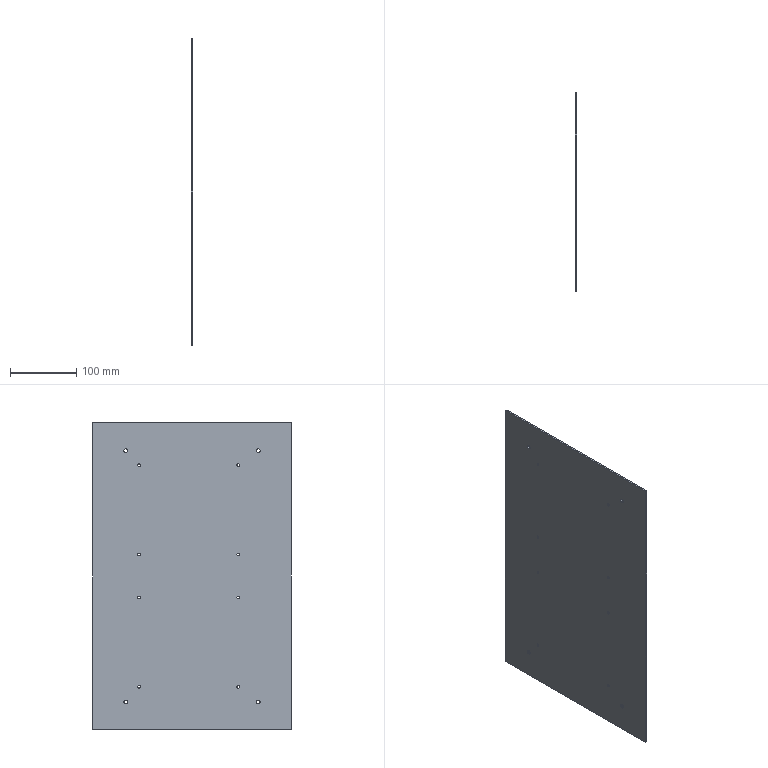Part | NX | features solid 2 | 1 solid | 50 faces | box 2.5 x 300 x 465 mm | volume 348190 mm3 | cylinder 44 | plane 6 | commonest cylinder face diameters 4.134 x32 6 x8 4 x4
STEP:
#1=CARTESIAN_POINT('',(-349.5,407.933,487.5));
#2=VERTEX_POINT('',#1);
#3=CARTESIAN_POINT('',(-347.5,407.933,487.5));
#4=VERTEX_POINT('',#3);
#5=CARTESIAN_POINT('',(203.882,407.933,487.5));
#6=DIRECTION('',(-1.,0.,0.));
#7=VECTOR('',#6,1000.);
#8=LINE('',#5,#7);
#9=EDGE_CURVE('',#2,#4,#8,.F.);
#10=ORIENTED_EDGE('',*,*,#9,.T.);
#11=CARTESIAN_POINT('',(-347.5,412.067,487.5));
#12=VERTEX_POINT('',#11);
#13=CARTESIAN_POINT('',(-347.5,410.,487.5));
#14=DIRECTION('',(-1.,0.,0.));
#15=DIRECTION('',(0.,1.,0.));
#16=AXIS2_PLACEMENT_3D('',#13,#14,#15);
#17=CIRCLE('',#16,2.067);
#18=EDGE_CURVE('',#12,#4,#17,.T.);
#19=ORIENTED_EDGE('',*,*,#18,.F.);
#20=CARTESIAN_POINT('',(-349.5,412.067,487.5));
#21=VERTEX_POINT('',#20);
#22=CARTESIAN_POINT('',(203.882,412.067,487.5));
#23=DIRECTION('',(-1.,0.,0.));
#24=VECTOR('',#23,1000.);
#25=LINE('',#22,#24);
#26=EDGE_CURVE('',#12,#21,#25,.T.);
#27=ORIENTED_EDGE('',*,*,#26,.T.);
#28=CARTESIAN_POINT('',(-349.5,410.,487.5));
#29=DIRECTION('',(-1.,0.,0.));
#30=DIRECTION('',(0.,1.,0.));
#31=AXIS2_PLACEMENT_3D('',#28,#29,#30);
#32=CIRCLE('',#31,2.067);
#33=EDGE_CURVE('',#21,#2,#32,.T.);
#34=ORIENTED_EDGE('',*,*,#33,.T.);
#35=EDGE_LOOP('',(#10,#19,#27,#34));
#36=FACE_BOUND('',#35,.T.);
#37=CARTESIAN_POINT('',(203.882,410.,487.5));
#38=DIRECTION('',(-1.,0.,0.));
#39=DIRECTION('',(0.,1.,0.));
#40=AXIS2_PLACEMENT_3D('',#37,#38,#39);
#41=CYLINDRICAL_SURFACE('',#40,2.067);
#42=ADVANCED_FACE('',(#36),#41,.F.);
#43=CARTESIAN_POINT('',(-347.5,407.933,352.5));
#44=VERTEX_POINT('',#43);
#45=CARTESIAN_POINT('',(-349.5,407.933,352.5));
#46=VERTEX_POINT('',#45);
#47=CARTESIAN_POINT('',(203.882,407.933,352.5));
#48=DIRECTION('',(-1.,0.,0.));
#49=VECTOR('',#48,1000.);
#50=LINE('',#47,#49);
#51=EDGE_CURVE('',#44,#46,#50,.T.);
#52=ORIENTED_EDGE('',*,*,#51,.F.);
#53=CARTESIAN_POINT('',(-347.5,412.067,352.5));
#54=VERTEX_POINT('',#53);
#55=CARTESIAN_POINT('',(-347.5,410.,352.5));
#56=DIRECTION('',(-1.,0.,0.));
#57=DIRECTION('',(0.,1.,0.));
#58=AXIS2_PLACEMENT_3D('',#55,#56,#57);
#59=CIRCLE('',#58,2.067);
#60=EDGE_CURVE('',#54,#44,#59,.T.);
#61=ORIENTED_EDGE('',*,*,#60,.F.);
#62=CARTESIAN_POINT('',(-349.5,412.067,352.5));
#63=VERTEX_POINT('',#62);
#64=CARTESIAN_POINT('',(203.882,412.067,352.5));
#65=DIRECTION('',(-1.,0.,0.));
#66=VECTOR('',#65,1000.);
#67=LINE('',#64,#66);
#68=EDGE_CURVE('',#63,#54,#67,.F.);
#69=ORIENTED_EDGE('',*,*,#68,.F.);
#70=CARTESIAN_POINT('',(-349.5,410.,352.5));
#71=DIRECTION('',(-1.,0.,0.));
#72=DIRECTION('',(0.,1.,0.));
#73=AXIS2_PLACEMENT_3D('',#70,#71,#72);
#74=CIRCLE('',#73,2.067);
#75=EDGE_CURVE('',#63,#46,#74,.T.);
#76=ORIENTED_EDGE('',*,*,#75,.T.);
#77=EDGE_LOOP('',(#52,#61,#69,#76));
#78=FACE_BOUND('',#77,.T.);
#79=CARTESIAN_POINT('',(203.882,410.,352.5));
#80=DIRECTION('',(-1.,0.,0.));
#81=DIRECTION('',(0.,1.,0.));
#82=AXIS2_PLACEMENT_3D('',#79,#80,#81);
#83=CYLINDRICAL_SURFACE('',#82,2.067);
#84=ADVANCED_FACE('',(#78),#83,.F.);
#85=CARTESIAN_POINT('',(-347.5,407.933,287.5));
#86=VERTEX_POINT('',#85);
#87=CARTESIAN_POINT('',(-349.5,407.933,287.5));
#88=VERTEX_POINT('',#87);
#89=CARTESIAN_POINT('',(203.882,407.933,287.5));
#90=DIRECTION('',(-1.,0.,0.));
#91=VECTOR('',#90,1000.);
#92=LINE('',#89,#91);
#93=EDGE_CURVE('',#86,#88,#92,.T.);
#94=ORIENTED_EDGE('',*,*,#93,.F.);
#95=CARTESIAN_POINT('',(-347.5,412.067,287.5));
#96=VERTEX_POINT('',#95);
#97=CARTESIAN_POINT('',(-347.5,410.,287.5));
#98=DIRECTION('',(-1.,0.,0.));
#99=DIRECTION('',(0.,1.,0.));
#100=AXIS2_PLACEMENT_3D('',#97,#98,#99);
#101=CIRCLE('',#100,2.067);
#102=EDGE_CURVE('',#96,#86,#101,.T.);
#103=ORIENTED_EDGE('',*,*,#102,.F.);
#104=CARTESIAN_POINT('',(-349.5,412.067,287.5));
#105=VERTEX_POINT('',#104);
#106=CARTESIAN_POINT('',(203.882,412.067,287.5));
#107=DIRECTION('',(-1.,0.,0.));
#108=VECTOR('',#107,1000.);
#109=LINE('',#106,#108);
#110=EDGE_CURVE('',#105,#96,#109,.F.);
#111=ORIENTED_EDGE('',*,*,#110,.F.);
#112=CARTESIAN_POINT('',(-349.5,410.,287.5));
#113=DIRECTION('',(-1.,0.,0.));
#114=DIRECTION('',(0.,1.,0.));
#115=AXIS2_PLACEMENT_3D('',#112,#113,#114);
#116=CIRCLE('',#115,2.067);
#117=EDGE_CURVE('',#105,#88,#116,.T.);
#118=ORIENTED_EDGE('',*,*,#117,.T.);
#119=EDGE_LOOP('',(#94,#103,#111,#118));
#120=FACE_BOUND('',#119,.T.);
#121=CARTESIAN_POINT('',(203.882,410.,287.5));
#122=DIRECTION('',(-1.,0.,0.));
#123=DIRECTION('',(0.,1.,0.));
#124=AXIS2_PLACEMENT_3D('',#121,#122,#123);
#125=CYLINDRICAL_SURFACE('',#124,2.067);
#126=ADVANCED_FACE('',(#120),#125,.F.);
#127=CARTESIAN_POINT('',(-347.5,257.933,487.5));
#128=VERTEX_POINT('',#127);
#129=CARTESIAN_POINT('',(-349.5,257.933,487.5));
#130=VERTEX_POINT('',#129);
#131=CARTESIAN_POINT('',(203.882,257.933,487.5));
#132=DIRECTION('',(-1.,0.,0.));
#133=VECTOR('',#132,1000.);
#134=LINE('',#131,#133);
#135=EDGE_CURVE('',#128,#130,#134,.T.);
#136=ORIENTED_EDGE('',*,*,#135,.F.);
#137=CARTESIAN_POINT('',(-347.5,262.067,487.5));
#138=VERTEX_POINT('',#137);
#139=CARTESIAN_POINT('',(-347.5,260.,487.5));
#140=DIRECTION('',(-1.,0.,0.));
#141=DIRECTION('',(0.,1.,0.));
#142=AXIS2_PLACEMENT_3D('',#139,#140,#141);
#143=CIRCLE('',#142,2.067);
#144=EDGE_CURVE('',#138,#128,#143,.T.);
#145=ORIENTED_EDGE('',*,*,#144,.F.);
#146=CARTESIAN_POINT('',(-349.5,262.067,487.5));
#147=VERTEX_POINT('',#146);
#148=CARTESIAN_POINT('',(203.882,262.067,487.5));
#149=DIRECTION('',(-1.,0.,0.));
#150=VECTOR('',#149,1000.);
#151=LINE('',#148,#150);
#152=EDGE_CURVE('',#147,#138,#151,.F.);
#153=ORIENTED_EDGE('',*,*,#152,.F.);
#154=CARTESIAN_POINT('',(-349.5,260.,487.5));
#155=DIRECTION('',(-1.,0.,0.));
#156=DIRECTION('',(0.,1.,0.));
#157=AXIS2_PLACEMENT_3D('',#154,#155,#156);
#158=CIRCLE('',#157,2.067);
#159=EDGE_CURVE('',#147,#130,#158,.T.);
#160=ORIENTED_EDGE('',*,*,#159,.T.);
#161=EDGE_LOOP('',(#136,#145,#153,#160));
#162=FACE_BOUND('',#161,.T.);
#163=CARTESIAN_POINT('',(203.882,260.,487.5));
#164=DIRECTION('',(-1.,0.,0.));
#165=DIRECTION('',(0.,1.,0.));
#166=AXIS2_PLACEMENT_3D('',#163,#164,#165);
#167=CYLINDRICAL_SURFACE('',#166,2.067);
#168=ADVANCED_FACE('',(#162),#167,.F.);
#169=CARTESIAN_POINT('',(-347.5,257.933,352.5));
#170=VERTEX_POINT('',#169);
#171=CARTESIAN_POINT('',(-349.5,257.933,352.5));
#172=VERTEX_POINT('',#171);
#173=CARTESIAN_POINT('',(203.882,257.933,352.5));
#174=DIRECTION('',(-1.,0.,0.));
#175=VECTOR('',#174,1000.);
#176=LINE('',#173,#175);
#177=EDGE_CURVE('',#170,#172,#176,.T.);
#178=ORIENTED_EDGE('',*,*,#177,.F.);
#179=CARTESIAN_POINT('',(-347.5,262.067,352.5));
#180=VERTEX_POINT('',#179);
#181=CARTESIAN_POINT('',(-347.5,260.,352.5));
#182=DIRECTION('',(-1.,0.,0.));
#183=DIRECTION('',(0.,1.,0.));
#184=AXIS2_PLACEMENT_3D('',#181,#182,#183);
#185=CIRCLE('',#184,2.067);
#186=EDGE_CURVE('',#180,#170,#185,.T.);
#187=ORIENTED_EDGE('',*,*,#186,.F.);
#188=CARTESIAN_POINT('',(-349.5,262.067,352.5));
#189=VERTEX_POINT('',#188);
#190=CARTESIAN_POINT('',(203.882,262.067,352.5));
#191=DIRECTION('',(-1.,0.,0.));
#192=VECTOR('',#191,1000.);
#193=LINE('',#190,#192);
#194=EDGE_CURVE('',#189,#180,#193,.F.);
#195=ORIENTED_EDGE('',*,*,#194,.F.);
#196=CARTESIAN_POINT('',(-349.5,260.,352.5));
#197=DIRECTION('',(-1.,0.,0.));
#198=DIRECTION('',(0.,1.,0.));
#199=AXIS2_PLACEMENT_3D('',#196,#197,#198);
#200=CIRCLE('',#199,2.067);
#201=EDGE_CURVE('',#189,#172,#200,.T.);
#202=ORIENTED_EDGE('',*,*,#201,.T.);
#203=EDGE_LOOP('',(#178,#187,#195,#202));
#204=FACE_BOUND('',#203,.T.);
#205=CARTESIAN_POINT('',(203.882,260.,352.5));
#206=DIRECTION('',(-1.,0.,0.));
#207=DIRECTION('',(0.,1.,0.));
#208=AXIS2_PLACEMENT_3D('',#205,#206,#207);
#209=CYLINDRICAL_SURFACE('',#208,2.067);
#210=ADVANCED_FACE('',(#204),#209,.F.);
#211=CARTESIAN_POINT('',(-347.5,257.933,287.5));
#212=VERTEX_POINT('',#211);
#213=CARTESIAN_POINT('',(-349.5,257.933,287.5));
#214=VERTEX_POINT('',#213);
#215=CARTESIAN_POINT('',(203.882,257.933,287.5));
#216=DIRECTION('',(-1.,0.,0.));
#217=VECTOR('',#216,1000.);
#218=LINE('',#215,#217);
#219=EDGE_CURVE('',#212,#214,#218,.T.);
#220=ORIENTED_EDGE('',*,*,#219,.F.);
#221=CARTESIAN_POINT('',(-347.5,262.067,287.5));
#222=VERTEX_POINT('',#221);
#223=CARTESIAN_POINT('',(-347.5,260.,287.5));
#224=DIRECTION('',(-1.,0.,0.));
#225=DIRECTION('',(0.,1.,0.));
#226=AXIS2_PLACEMENT_3D('',#223,#224,#225);
#227=CIRCLE('',#226,2.067);
#228=EDGE_CURVE('',#222,#212,#227,.T.);
#229=ORIENTED_EDGE('',*,*,#228,.F.);
#230=CARTESIAN_POINT('',(-349.5,262.067,287.5));
#231=VERTEX_POINT('',#230);
#232=CARTESIAN_POINT('',(203.882,262.067,287.5));
#233=DIRECTION('',(-1.,0.,0.));
#234=VECTOR('',#233,1000.);
#235=LINE('',#232,#234);
#236=EDGE_CURVE('',#231,#222,#235,.F.);
#237=ORIENTED_EDGE('',*,*,#236,.F.);
#238=CARTESIAN_POINT('',(-349.5,260.,287.5));
#239=DIRECTION('',(-1.,0.,0.));
#240=DIRECTION('',(0.,1.,0.));
#241=AXIS2_PLACEMENT_3D('',#238,#239,#240);
#242=CIRCLE('',#241,2.067);
#243=EDGE_CURVE('',#231,#214,#242,.T.);
#244=ORIENTED_EDGE('',*,*,#243,.T.);
#245=EDGE_LOOP('',(#220,#229,#237,#244));
#246=FACE_BOUND('',#245,.T.);
#247=CARTESIAN_POINT('',(203.882,260.,287.5));
#248=DIRECTION('',(-1.,0.,0.));
#249=DIRECTION('',(0.,1.,0.));
#250=AXIS2_PLACEMENT_3D('',#247,#248,#249);
#251=CYLINDRICAL_SURFACE('',#250,2.067);
#252=ADVANCED_FACE('',(#246),#251,.F.);
#253=CARTESIAN_POINT('',(-347.5,407.933,152.5));
#254=VERTEX_POINT('',#253);
#255=CARTESIAN_POINT('',(-349.5,407.933,152.5));
#256=VERTEX_POINT('',#255);
#257=CARTESIAN_POINT('',(203.882,407.933,152.5));
#258=DIRECTION('',(-1.,0.,0.));
#259=VECTOR('',#258,1000.);
#260=LINE('',#257,#259);
#261=EDGE_CURVE('',#254,#256,#260,.T.);
#262=ORIENTED_EDGE('',*,*,#261,.F.);
#263=CARTESIAN_POINT('',(-347.5,412.067,152.5));
#264=VERTEX_POINT('',#263);
#265=CARTESIAN_POINT('',(-347.5,410.,152.5));
#266=DIRECTION('',(-1.,0.,0.));
#267=DIRECTION('',(0.,1.,0.));
#268=AXIS2_PLACEMENT_3D('',#265,#266,#267);
#269=CIRCLE('',#268,2.067);
#270=EDGE_CURVE('',#264,#254,#269,.T.);
#271=ORIENTED_EDGE('',*,*,#270,.F.);
#272=CARTESIAN_POINT('',(-349.5,412.067,152.5));
#273=VERTEX_POINT('',#272);
#274=CARTESIAN_POINT('',(203.882,412.067,152.5));
#275=DIRECTION('',(-1.,0.,0.));
#276=VECTOR('',#275,1000.);
#277=LINE('',#274,#276);
#278=EDGE_CURVE('',#273,#264,#277,.F.);
#279=ORIENTED_EDGE('',*,*,#278,.F.);
#280=CARTESIAN_POINT('',(-349.5,410.,152.5));
#281=DIRECTION('',(-1.,0.,0.));
#282=DIRECTION('',(0.,1.,0.));
#283=AXIS2_PLACEMENT_3D('',#280,#281,#282);
#284=CIRCLE('',#283,2.067);
#285=EDGE_CURVE('',#273,#256,#284,.T.);
#286=ORIENTED_EDGE('',*,*,#285,.T.);
#287=EDGE_LOOP('',(#262,#271,#279,#286));
#288=FACE_BOUND('',#287,.T.);
#289=CARTESIAN_POINT('',(203.882,410.,152.5));
#290=DIRECTION('',(-1.,0.,0.));
#291=DIRECTION('',(0.,1.,0.));
#292=AXIS2_PLACEMENT_3D('',#289,#290,#291);
#293=CYLINDRICAL_SURFACE('',#292,2.067);
#294=ADVANCED_FACE('',(#288),#293,.F.);
#295=CARTESIAN_POINT('',(-347.5,257.933,152.5));
#296=VERTEX_POINT('',#295);
#297=CARTESIAN_POINT('',(-349.5,257.933,152.5));
#298=VERTEX_POINT('',#297);
#299=CARTESIAN_POINT('',(203.882,257.933,152.5));
#300=DIRECTION('',(-1.,0.,0.));
#301=VECTOR('',#300,1000.);
#302=LINE('',#299,#301);
#303=EDGE_CURVE('',#296,#298,#302,.T.);
#304=ORIENTED_EDGE('',*,*,#303,.F.);
#305=CARTESIAN_POINT('',(-347.5,262.067,152.5));
#306=VERTEX_POINT('',#305);
#307=CARTESIAN_POINT('',(-347.5,260.,152.5));
#308=DIRECTION('',(-1.,0.,0.));
#309=DIRECTION('',(0.,1.,0.));
#310=AXIS2_PLACEMENT_3D('',#307,#308,#309);
#311=CIRCLE('',#310,2.067);
#312=EDGE_CURVE('',#306,#296,#311,.T.);
#313=ORIENTED_EDGE('',*,*,#312,.F.);
#314=CARTESIAN_POINT('',(-349.5,262.067,152.5));
#315=VERTEX_POINT('',#314);
#316=CARTESIAN_POINT('',(203.882,262.067,152.5));
#317=DIRECTION('',(-1.,0.,0.));
#318=VECTOR('',#317,1000.);
#319=LINE('',#316,#318);
#320=EDGE_CURVE('',#315,#306,#319,.F.);
#321=ORIENTED_EDGE('',*,*,#320,.F.);
#322=CARTESIAN_POINT('',(-349.5,260.,152.5));
#323=DIRECTION('',(-1.,0.,0.));
#324=DIRECTION('',(0.,1.,0.));
#325=AXIS2_PLACEMENT_3D('',#322,#323,#324);
#326=CIRCLE('',#325,2.067);
#327=EDGE_CURVE('',#315,#298,#326,.T.);
#328=ORIENTED_EDGE('',*,*,#327,.T.);
#329=EDGE_LOOP('',(#304,#313,#321,#328));
#330=FACE_BOUND('',#329,.T.);
#331=CARTESIAN_POINT('',(203.882,260.,152.5));
#332=DIRECTION('',(-1.,0.,0.));
#333=DIRECTION('',(0.,1.,0.));
#334=AXIS2_PLACEMENT_3D('',#331,#332,#333);
#335=CYLINDRICAL_SURFACE('',#334,2.067);
#336=ADVANCED_FACE('',(#330),#335,.F.);
#337=CARTESIAN_POINT('',(-347.,227.,509.5));
#338=VERTEX_POINT('',#337);
#339=CARTESIAN_POINT('',(-349.5,227.,509.5));
#340=VERTEX_POINT('',#339);
#341=CARTESIAN_POINT('',(203.882,227.,509.5));
#342=DIRECTION('',(-1.,0.,0.));
#343=VECTOR('',#342,1000.);
#344=LINE('',#341,#343);
#345=EDGE_CURVE('',#338,#340,#344,.T.);
#346=ORIENTED_EDGE('',*,*,#345,.F.);
#347=CARTESIAN_POINT('',(-347.,233.,509.5));
#348=VERTEX_POINT('',#347);
#349=CARTESIAN_POINT('',(-347.,230.,509.5));
#350=DIRECTION('',(-1.,0.,0.));
#351=DIRECTION('',(0.,1.,0.));
#352=AXIS2_PLACEMENT_3D('',#349,#350,#351);
#353=CIRCLE('',#352,3.);
#354=EDGE_CURVE('',#348,#338,#353,.T.);
#355=ORIENTED_EDGE('',*,*,#354,.F.);
#356=CARTESIAN_POINT('',(-349.5,233.,509.5));
#357=VERTEX_POINT('',#356);
#358=CARTESIAN_POINT('',(203.882,233.,509.5));
#359=DIRECTION('',(-1.,0.,0.));
#360=VECTOR('',#359,1000.);
#361=LINE('',#358,#360);
#362=EDGE_CURVE('',#357,#348,#361,.F.);
#363=ORIENTED_EDGE('',*,*,#362,.F.);
#364=CARTESIAN_POINT('',(-349.5,230.,509.5));
#365=DIRECTION('',(-1.,0.,0.));
#366=DIRECTION('',(0.,1.,0.));
#367=AXIS2_PLACEMENT_3D('',#364,#365,#366);
#368=CIRCLE('',#367,3.);
#369=EDGE_CURVE('',#357,#340,#368,.T.);
#370=ORIENTED_EDGE('',*,*,#369,.T.);
#371=EDGE_LOOP('',(#346,#355,#363,#370));
#372=FACE_BOUND('',#371,.T.);
#373=CARTESIAN_POINT('',(203.882,230.,509.5));
#374=DIRECTION('',(-1.,0.,0.));
#375=DIRECTION('',(0.,1.,0.));
#376=AXIS2_PLACEMENT_3D('',#373,#374,#375);
#377=CYLINDRICAL_SURFACE('',#376,3.);
#378=ADVANCED_FACE('',(#372),#377,.F.);
#379=CARTESIAN_POINT('',(-347.,427.,509.5));
#380=VERTEX_POINT('',#379);
#381=CARTESIAN_POINT('',(-349.5,427.,509.5));
#382=VERTEX_POINT('',#381);
#383=CARTESIAN_POINT('',(203.882,427.,509.5));
#384=DIRECTION('',(-1.,0.,0.));
#385=VECTOR('',#384,1000.);
#386=LINE('',#383,#385);
#387=EDGE_CURVE('',#380,#382,#386,.T.);
#388=ORIENTED_EDGE('',*,*,#387,.F.);
#389=CARTESIAN_POINT('',(-347.,433.,509.5));
#390=VERTEX_POINT('',#389);
#391=CARTESIAN_POINT('',(-347.,430.,509.5));
#392=DIRECTION('',(-1.,0.,0.));
#393=DIRECTION('',(0.,1.,0.));
#394=AXIS2_PLACEMENT_3D('',#391,#392,#393);
#395=CIRCLE('',#394,3.);
#396=EDGE_CURVE('',#390,#380,#395,.T.);
#397=ORIENTED_EDGE('',*,*,#396,.F.);
#398=CARTESIAN_POINT('',(-349.5,433.,509.5));
#399=VERTEX_POINT('',#398);
#400=CARTESIAN_POINT('',(203.882,433.,509.5));
#401=DIRECTION('',(-1.,0.,0.));
#402=VECTOR('',#401,1000.);
#403=LINE('',#400,#402);
#404=EDGE_CURVE('',#399,#390,#403,.F.);
#405=ORIENTED_EDGE('',*,*,#404,.F.);
#406=CARTESIAN_POINT('',(-349.5,430.,509.5));
#407=DIRECTION('',(-1.,0.,0.));
#408=DIRECTION('',(0.,1.,0.));
#409=AXIS2_PLACEMENT_3D('',#406,#407,#408);
#410=CIRCLE('',#409,3.);
#411=EDGE_CURVE('',#399,#382,#410,.T.);
#412=ORIENTED_EDGE('',*,*,#411,.T.);
#413=EDGE_LOOP('',(#388,#397,#405,#412));
#414=FACE_BOUND('',#413,.T.);
#415=CARTESIAN_POINT('',(203.882,430.,509.5));
#416=DIRECTION('',(-1.,0.,0.));
#417=DIRECTION('',(0.,1.,0.));
#418=AXIS2_PLACEMENT_3D('',#415,#416,#417);
#419=CYLINDRICAL_SURFACE('',#418,3.);
#420=ADVANCED_FACE('',(#414),#419,.F.);
#421=CARTESIAN_POINT('',(-347.,427.,129.5));
#422=VERTEX_POINT('',#421);
#423=CARTESIAN_POINT('',(-349.5,427.,129.5));
#424=VERTEX_POINT('',#423);
#425=CARTESIAN_POINT('',(203.882,427.,129.5));
#426=DIRECTION('',(-1.,0.,0.));
#427=VECTOR('',#426,1000.);
#428=LINE('',#425,#427);
#429=EDGE_CURVE('',#422,#424,#428,.T.);
#430=ORIENTED_EDGE('',*,*,#429,.F.);
#431=CARTESIAN_POINT('',(-347.,433.,129.5));
#432=VERTEX_POINT('',#431);
#433=CARTESIAN_POINT('',(-347.,430.,129.5));
#434=DIRECTION('',(-1.,0.,0.));
#435=DIRECTION('',(0.,1.,0.));
#436=AXIS2_PLACEMENT_3D('',#433,#434,#435);
#437=CIRCLE('',#436,3.);
#438=EDGE_CURVE('',#432,#422,#437,.T.);
#439=ORIENTED_EDGE('',*,*,#438,.F.);
#440=CARTESIAN_POINT('',(-349.5,433.,129.5));
#441=VERTEX_POINT('',#440);
#442=CARTESIAN_POINT('',(203.882,433.,129.5));
#443=DIRECTION('',(-1.,0.,0.));
#444=VECTOR('',#443,1000.);
#445=LINE('',#442,#444);
#446=EDGE_CURVE('',#441,#432,#445,.F.);
#447=ORIENTED_EDGE('',*,*,#446,.F.);
#448=CARTESIAN_POINT('',(-349.5,430.,129.5));
#449=DIRECTION('',(-1.,0.,0.));
#450=DIRECTION('',(0.,1.,0.));
#451=AXIS2_PLACEMENT_3D('',#448,#449,#450);
#452=CIRCLE('',#451,3.);
#453=EDGE_CURVE('',#441,#424,#452,.T.);
#454=ORIENTED_EDGE('',*,*,#453,.T.);
#455=EDGE_LOOP('',(#430,#439,#447,#454));
#456=FACE_BOUND('',#455,.T.);
#457=CARTESIAN_POINT('',(203.882,430.,129.5));
#458=DIRECTION('',(-1.,0.,0.));
#459=DIRECTION('',(0.,1.,0.));
#460=AXIS2_PLACEMENT_3D('',#457,#458,#459);
#461=CYLINDRICAL_SURFACE('',#460,3.);
#462=ADVANCED_FACE('',(#456),#461,.F.);
#463=CARTESIAN_POINT('',(-347.,227.,129.5));
#464=VERTEX_POINT('',#463);
#465=CARTESIAN_POINT('',(-349.5,227.,129.5));
#466=VERTEX_POINT('',#465);
#467=CARTESIAN_POINT('',(203.882,227.,129.5));
#468=DIRECTION('',(-1.,0.,0.));
#469=VECTOR('',#468,1000.);
#470=LINE('',#467,#469);
#471=EDGE_CURVE('',#464,#466,#470,.T.);
#472=ORIENTED_EDGE('',*,*,#471,.F.);
#473=CARTESIAN_POINT('',(-347.,233.,129.5));
#474=VERTEX_POINT('',#473);
#475=CARTESIAN_POINT('',(-347.,230.,129.5));
#476=DIRECTION('',(-1.,0.,0.));
#477=DIRECTION('',(0.,1.,0.));
#478=AXIS2_PLACEMENT_3D('',#475,#476,#477);
#479=CIRCLE('',#478,3.);
#480=EDGE_CURVE('',#474,#464,#479,.T.);
#481=ORIENTED_EDGE('',*,*,#480,.F.);
#482=CARTESIAN_POINT('',(-349.5,233.,129.5));
#483=VERTEX_POINT('',#482);
#484=CARTESIAN_POINT('',(203.882,233.,129.5));
#485=DIRECTION('',(-1.,0.,0.));
#486=VECTOR('',#485,1000.);
#487=LINE('',#484,#486);
#488=EDGE_CURVE('',#483,#474,#487,.F.);
#489=ORIENTED_EDGE('',*,*,#488,.F.);
#490=CARTESIAN_POINT('',(-349.5,230.,129.5));
#491=DIRECTION('',(-1.,0.,0.));
#492=DIRECTION('',(0.,1.,0.));
#493=AXIS2_PLACEMENT_3D('',#490,#491,#492);
#494=CIRCLE('',#493,3.);
#495=EDGE_CURVE('',#483,#466,#494,.T.);
#496=ORIENTED_EDGE('',*,*,#495,.T.);
#497=EDGE_LOOP('',(#472,#481,#489,#496));
#498=FACE_BOUND('',#497,.T.);
#499=CARTESIAN_POINT('',(203.882,230.,129.5));
#500=DIRECTION('',(-1.,0.,0.));
#501=DIRECTION('',(0.,1.,0.));
#502=AXIS2_PLACEMENT_3D('',#499,#500,#501);
#503=CYLINDRICAL_SURFACE('',#502,3.);
#504=ADVANCED_FACE('',(#498),#503,.F.);
#505=CARTESIAN_POINT('',(-347.,478.,87.5));
#506=VERTEX_POINT('',#505);
#507=CARTESIAN_POINT('',(-347.,480.,89.5));
#508=VERTEX_POINT('',#507);
#509=CARTESIAN_POINT('',(-347.,478.,89.5));
#510=DIRECTION('',(1.,0.,0.));
#511=DIRECTION('',(0.,1.,0.));
#512=AXIS2_PLACEMENT_3D('',#509,#510,#511);
#513=CIRCLE('',#512,2.);
#514=EDGE_CURVE('',#506,#508,#513,.T.);
#515=ORIENTED_EDGE('',*,*,#514,.F.);
#516=CARTESIAN_POINT('',(-349.5,478.,87.5));
#517=VERTEX_POINT('',#516);
#518=CARTESIAN_POINT('',(-347.,478.,87.5));
#519=DIRECTION('',(1.,0.,0.));
#520=VECTOR('',#519,1000.);
#521=LINE('',#518,#520);
#522=EDGE_CURVE('',#517,#506,#521,.T.);
#523=ORIENTED_EDGE('',*,*,#522,.F.);
#524=CARTESIAN_POINT('',(-349.5,480.,89.5));
#525=VERTEX_POINT('',#524);
#526=CARTESIAN_POINT('',(-349.5,478.,89.5));
#527=DIRECTION('',(-1.,0.,0.));
#528=DIRECTION('',(0.,1.,0.));
#529=AXIS2_PLACEMENT_3D('',#526,#527,#528);
#530=CIRCLE('',#529,2.);
#531=EDGE_CURVE('',#525,#517,#530,.T.);
#532=ORIENTED_EDGE('',*,*,#531,.F.);
#533=CARTESIAN_POINT('',(-347.,480.,89.5));
#534=DIRECTION('',(-1.,0.,0.));
#535=VECTOR('',#534,1000.);
#536=LINE('',#533,#535);
#537=EDGE_CURVE('',#508,#525,#536,.T.);
#538=ORIENTED_EDGE('',*,*,#537,.F.);
#539=EDGE_LOOP('',(#515,#523,#532,#538));
#540=FACE_BOUND('',#539,.T.);
#541=CARTESIAN_POINT('',(-347.,478.,89.5));
#542=DIRECTION('',(-1.,0.,0.));
#543=DIRECTION('',(0.,0.,1.));
#544=AXIS2_PLACEMENT_3D('',#541,#542,#543);
#545=CYLINDRICAL_SURFACE('',#544,2.);
#546=ADVANCED_FACE('',(#540),#545,.T.);
#547=CARTESIAN_POINT('',(-347.,480.,550.5));
#548=VERTEX_POINT('',#547);
#549=CARTESIAN_POINT('',(-347.,478.,552.5));
#550=VERTEX_POINT('',#549);
#551=CARTESIAN_POINT('',(-347.,478.,550.5));
#552=DIRECTION('',(1.,0.,0.));
#553=DIRECTION('',(0.,1.,0.));
#554=AXIS2_PLACEMENT_3D('',#551,#552,#553);
#555=CIRCLE('',#554,2.);
#556=EDGE_CURVE('',#548,#550,#555,.T.);
#557=ORIENTED_EDGE('',*,*,#556,.F.);
#558=CARTESIAN_POINT('',(-349.5,480.,550.5));
#559=VERTEX_POINT('',#558);
#560=CARTESIAN_POINT('',(-347.,480.,550.5));
#561=DIRECTION('',(1.,0.,0.));
#562=VECTOR('',#561,1000.);
#563=LINE('',#560,#562);
#564=EDGE_CURVE('',#559,#548,#563,.T.);
#565=ORIENTED_EDGE('',*,*,#564,.F.);
#566=CARTESIAN_POINT('',(-349.5,478.,552.5));
#567=VERTEX_POINT('',#566);
#568=CARTESIAN_POINT('',(-349.5,478.,550.5));
#569=DIRECTION('',(-1.,0.,0.));
#570=DIRECTION('',(0.,1.,0.));
#571=AXIS2_PLACEMENT_3D('',#568,#569,#570);
#572=CIRCLE('',#571,2.);
#573=EDGE_CURVE('',#567,#559,#572,.T.);
#574=ORIENTED_EDGE('',*,*,#573,.F.);
#575=CARTESIAN_POINT('',(-347.,478.,552.5));
#576=DIRECTION('',(-1.,0.,0.));
#577=VECTOR('',#576,1000.);
#578=LINE('',#575,#577);
#579=EDGE_CURVE('',#550,#567,#578,.T.);
#580=ORIENTED_EDGE('',*,*,#579,.F.);
#581=EDGE_LOOP('',(#557,#565,#574,#580));
#582=FACE_BOUND('',#581,.T.);
#583=CARTESIAN_POINT('',(-347.,478.,550.5));
#584=DIRECTION('',(-1.,0.,0.));
#585=DIRECTION('',(0.,0.,1.));
#586=AXIS2_PLACEMENT_3D('',#583,#584,#585);
#587=CYLINDRICAL_SURFACE('',#586,2.);
#588=ADVANCED_FACE('',(#582),#587,.T.);
#589=CARTESIAN_POINT('',(-347.,182.,552.5));
#590=VERTEX_POINT('',#589);
#591=CARTESIAN_POINT('',(-347.,180.,550.5));
#592=VERTEX_POINT('',#591);
#593=CARTESIAN_POINT('',(-347.,182.,550.5));
#594=DIRECTION('',(1.,0.,0.));
#595=DIRECTION('',(0.,1.,0.));
#596=AXIS2_PLACEMENT_3D('',#593,#594,#595);
#597=CIRCLE('',#596,2.);
#598=EDGE_CURVE('',#590,#592,#597,.T.);
#599=ORIENTED_EDGE('',*,*,#598,.F.);
#600=CARTESIAN_POINT('',(-349.5,182.,552.5));
#601=VERTEX_POINT('',#600);
#602=CARTESIAN_POINT('',(-347.,182.,552.5));
#603=DIRECTION('',(1.,0.,0.));
#604=VECTOR('',#603,1000.);
#605=LINE('',#602,#604);
#606=EDGE_CURVE('',#601,#590,#605,.T.);
#607=ORIENTED_EDGE('',*,*,#606,.F.);
#608=CARTESIAN_POINT('',(-349.5,180.,550.5));
#609=VERTEX_POINT('',#608);
#610=CARTESIAN_POINT('',(-349.5,182.,550.5));
#611=DIRECTION('',(-1.,0.,0.));
#612=DIRECTION('',(0.,1.,0.));
#613=AXIS2_PLACEMENT_3D('',#610,#611,#612);
#614=CIRCLE('',#613,2.);
#615=EDGE_CURVE('',#609,#601,#614,.T.);
#616=ORIENTED_EDGE('',*,*,#615,.F.);
#617=CARTESIAN_POINT('',(-347.,180.,550.5));
#618=DIRECTION('',(-1.,0.,0.));
#619=VECTOR('',#618,1000.);
#620=LINE('',#617,#619);
#621=EDGE_CURVE('',#592,#609,#620,.T.);
#622=ORIENTED_EDGE('',*,*,#621,.F.);
#623=EDGE_LOOP('',(#599,#607,#616,#622));
#624=FACE_BOUND('',#623,.T.);
#625=CARTESIAN_POINT('',(-347.,182.,550.5));
#626=DIRECTION('',(-1.,0.,0.));
#627=DIRECTION('',(0.,0.,1.));
#628=AXIS2_PLACEMENT_3D('',#625,#626,#627);
#629=CYLINDRICAL_SURFACE('',#628,2.);
#630=ADVANCED_FACE('',(#624),#629,.T.);
#631=CARTESIAN_POINT('',(-347.,180.,89.5));
#632=VERTEX_POINT('',#631);
#633=CARTESIAN_POINT('',(-347.,182.,87.5));
#634=VERTEX_POINT('',#633);
#635=CARTESIAN_POINT('',(-347.,182.,89.5));
#636=DIRECTION('',(1.,0.,0.));
#637=DIRECTION('',(0.,1.,0.));
#638=AXIS2_PLACEMENT_3D('',#635,#636,#637);
#639=CIRCLE('',#638,2.);
#640=EDGE_CURVE('',#632,#634,#639,.T.);
#641=ORIENTED_EDGE('',*,*,#640,.F.);
#642=CARTESIAN_POINT('',(-349.5,180.,89.5));
#643=VERTEX_POINT('',#642);
#644=CARTESIAN_POINT('',(-347.,180.,89.5));
#645=DIRECTION('',(1.,0.,0.));
#646=VECTOR('',#645,1000.);
#647=LINE('',#644,#646);
#648=EDGE_CURVE('',#643,#632,#647,.T.);
#649=ORIENTED_EDGE('',*,*,#648,.F.);
#650=CARTESIAN_POINT('',(-349.5,182.,87.5));
#651=VERTEX_POINT('',#650);
#652=CARTESIAN_POINT('',(-349.5,182.,89.5));
#653=DIRECTION('',(-1.,0.,0.));
#654=DIRECTION('',(0.,1.,0.));
#655=AXIS2_PLACEMENT_3D('',#652,#653,#654);
#656=CIRCLE('',#655,2.);
#657=EDGE_CURVE('',#651,#643,#656,.T.);
#658=ORIENTED_EDGE('',*,*,#657,.F.);
#659=CARTESIAN_POINT('',(-347.,182.,87.5));
#660=DIRECTION('',(-1.,0.,0.));
#661=VECTOR('',#660,1000.);
#662=LINE('',#659,#661);
#663=EDGE_CURVE('',#634,#651,#662,.T.);
#664=ORIENTED_EDGE('',*,*,#663,.F.);
#665=EDGE_LOOP('',(#641,#649,#658,#664));
#666=FACE_BOUND('',#665,.T.);
#667=CARTESIAN_POINT('',(-347.,182.,89.5));
#668=DIRECTION('',(-1.,0.,0.));
#669=DIRECTION('',(0.,0.,1.));
#670=AXIS2_PLACEMENT_3D('',#667,#668,#669);
#671=CYLINDRICAL_SURFACE('',#670,2.);
#672=ADVANCED_FACE('',(#666),#671,.T.);
#673=ORIENTED_EDGE('',*,*,#495,.F.);
#674=CARTESIAN_POINT('',(-349.5,230.,129.5));
#675=DIRECTION('',(-1.,0.,0.));
#676=DIRECTION('',(0.,1.,0.));
#677=AXIS2_PLACEMENT_3D('',#674,#675,#676);
#678=CIRCLE('',#677,3.);
#679=EDGE_CURVE('',#466,#483,#678,.T.);
#680=ORIENTED_EDGE('',*,*,#679,.F.);
#681=EDGE_LOOP('',(#673,#680));
#682=FACE_BOUND('',#681,.T.);
#683=ORIENTED_EDGE('',*,*,#453,.F.);
#684=CARTESIAN_POINT('',(-349.5,430.,129.5));
#685=DIRECTION('',(-1.,0.,0.));
#686=DIRECTION('',(0.,1.,0.));
#687=AXIS2_PLACEMENT_3D('',#684,#685,#686);
#688=CIRCLE('',#687,3.);
#689=EDGE_CURVE('',#424,#441,#688,.T.);
#690=ORIENTED_EDGE('',*,*,#689,.F.);
#691=EDGE_LOOP('',(#683,#690));
#692=FACE_BOUND('',#691,.T.);
#693=ORIENTED_EDGE('',*,*,#411,.F.);
#694=CARTESIAN_POINT('',(-349.5,430.,509.5));
#695=DIRECTION('',(-1.,0.,0.));
#696=DIRECTION('',(0.,1.,0.));
#697=AXIS2_PLACEMENT_3D('',#694,#695,#696);
#698=CIRCLE('',#697,3.);
#699=EDGE_CURVE('',#382,#399,#698,.T.);
#700=ORIENTED_EDGE('',*,*,#699,.F.);
#701=EDGE_LOOP('',(#693,#700));
#702=FACE_BOUND('',#701,.T.);
#703=ORIENTED_EDGE('',*,*,#369,.F.);
#704=CARTESIAN_POINT('',(-349.5,230.,509.5));
#705=DIRECTION('',(-1.,0.,0.));
#706=DIRECTION('',(0.,1.,0.));
#707=AXIS2_PLACEMENT_3D('',#704,#705,#706);
#708=CIRCLE('',#707,3.);
#709=EDGE_CURVE('',#340,#357,#708,.T.);
#710=ORIENTED_EDGE('',*,*,#709,.F.);
#711=EDGE_LOOP('',(#703,#710));
#712=FACE_BOUND('',#711,.T.);
#713=ORIENTED_EDGE('',*,*,#327,.F.);
#714=CARTESIAN_POINT('',(-349.5,260.,152.5));
#715=DIRECTION('',(-1.,0.,0.));
#716=DIRECTION('',(0.,1.,0.));
#717=AXIS2_PLACEMENT_3D('',#714,#715,#716);
#718=CIRCLE('',#717,2.067);
#719=EDGE_CURVE('',#298,#315,#718,.T.);
#720=ORIENTED_EDGE('',*,*,#719,.F.);
#721=EDGE_LOOP('',(#713,#720));
#722=FACE_BOUND('',#721,.T.);
#723=ORIENTED_EDGE('',*,*,#285,.F.);
#724=CARTESIAN_POINT('',(-349.5,410.,152.5));
#725=DIRECTION('',(-1.,0.,0.));
#726=DIRECTION('',(0.,1.,0.));
#727=AXIS2_PLACEMENT_3D('',#724,#725,#726);
#728=CIRCLE('',#727,2.067);
#729=EDGE_CURVE('',#256,#273,#728,.T.);
#730=ORIENTED_EDGE('',*,*,#729,.F.);
#731=EDGE_LOOP('',(#723,#730));
#732=FACE_BOUND('',#731,.T.);
#733=ORIENTED_EDGE('',*,*,#243,.F.);
#734=CARTESIAN_POINT('',(-349.5,260.,287.5));
#735=DIRECTION('',(-1.,0.,0.));
#736=DIRECTION('',(0.,1.,0.));
#737=AXIS2_PLACEMENT_3D('',#734,#735,#736);
#738=CIRCLE('',#737,2.067);
#739=EDGE_CURVE('',#214,#231,#738,.T.);
#740=ORIENTED_EDGE('',*,*,#739,.F.);
#741=EDGE_LOOP('',(#733,#740));
#742=FACE_BOUND('',#741,.T.);
#743=ORIENTED_EDGE('',*,*,#201,.F.);
#744=CARTESIAN_POINT('',(-349.5,260.,352.5));
#745=DIRECTION('',(-1.,0.,0.));
#746=DIRECTION('',(0.,1.,0.));
#747=AXIS2_PLACEMENT_3D('',#744,#745,#746);
#748=CIRCLE('',#747,2.067);
#749=EDGE_CURVE('',#172,#189,#748,.T.);
#750=ORIENTED_EDGE('',*,*,#749,.F.);
#751=EDGE_LOOP('',(#743,#750));
#752=FACE_BOUND('',#751,.T.);
#753=ORIENTED_EDGE('',*,*,#159,.F.);
#754=CARTESIAN_POINT('',(-349.5,260.,487.5));
#755=DIRECTION('',(-1.,0.,0.));
#756=DIRECTION('',(0.,1.,0.));
#757=AXIS2_PLACEMENT_3D('',#754,#755,#756);
#758=CIRCLE('',#757,2.067);
#759=EDGE_CURVE('',#130,#147,#758,.T.);
#760=ORIENTED_EDGE('',*,*,#759,.F.);
#761=EDGE_LOOP('',(#753,#760));
#762=FACE_BOUND('',#761,.T.);
#763=ORIENTED_EDGE('',*,*,#117,.F.);
#764=CARTESIAN_POINT('',(-349.5,410.,287.5));
#765=DIRECTION('',(-1.,0.,0.));
#766=DIRECTION('',(0.,1.,0.));
#767=AXIS2_PLACEMENT_3D('',#764,#765,#766);
#768=CIRCLE('',#767,2.067);
#769=EDGE_CURVE('',#88,#105,#768,.T.);
#770=ORIENTED_EDGE('',*,*,#769,.F.);
#771=EDGE_LOOP('',(#763,#770));
#772=FACE_BOUND('',#771,.T.);
#773=ORIENTED_EDGE('',*,*,#75,.F.);
#774=CARTESIAN_POINT('',(-349.5,410.,352.5));
#775=DIRECTION('',(-1.,0.,0.));
#776=DIRECTION('',(0.,1.,0.));
#777=AXIS2_PLACEMENT_3D('',#774,#775,#776);
#778=CIRCLE('',#777,2.067);
#779=EDGE_CURVE('',#46,#63,#778,.T.);
#780=ORIENTED_EDGE('',*,*,#779,.F.);
#781=EDGE_LOOP('',(#773,#780));
#782=FACE_BOUND('',#781,.T.);
#783=ORIENTED_EDGE('',*,*,#33,.F.);
#784=CARTESIAN_POINT('',(-349.5,410.,487.5));
#785=DIRECTION('',(-1.,0.,0.));
#786=DIRECTION('',(0.,1.,0.));
#787=AXIS2_PLACEMENT_3D('',#784,#785,#786);
#788=CIRCLE('',#787,2.067);
#789=EDGE_CURVE('',#2,#21,#788,.T.);
#790=ORIENTED_EDGE('',*,*,#789,.F.);
#791=EDGE_LOOP('',(#783,#790));
#792=FACE_BOUND('',#791,.T.);
#793=CARTESIAN_POINT('',(-349.5,180.,87.5));
#794=DIRECTION('',(0.,0.,1.));
#795=VECTOR('',#794,1000.);
#796=LINE('',#793,#795);
#797=EDGE_CURVE('',#643,#609,#796,.T.);
#798=ORIENTED_EDGE('',*,*,#797,.T.);
#799=ORIENTED_EDGE('',*,*,#615,.T.);
#800=CARTESIAN_POINT('',(-349.5,180.,552.5));
#801=DIRECTION('',(0.,1.,0.));
#802=VECTOR('',#801,1000.);
#803=LINE('',#800,#802);
#804=EDGE_CURVE('',#601,#567,#803,.T.);
#805=ORIENTED_EDGE('',*,*,#804,.T.);
#806=ORIENTED_EDGE('',*,*,#573,.T.);
#807=CARTESIAN_POINT('',(-349.5,480.,552.5));
#808=DIRECTION('',(0.,0.,-1.));
#809=VECTOR('',#808,1000.);
#810=LINE('',#807,#809);
#811=EDGE_CURVE('',#559,#525,#810,.T.);
#812=ORIENTED_EDGE('',*,*,#811,.T.);
#813=ORIENTED_EDGE('',*,*,#531,.T.);
#814=CARTESIAN_POINT('',(-349.5,480.,87.5));
#815=DIRECTION('',(0.,-1.,0.));
#816=VECTOR('',#815,1000.);
#817=LINE('',#814,#816);
#818=EDGE_CURVE('',#517,#651,#817,.T.);
#819=ORIENTED_EDGE('',*,*,#818,.T.);
#820=ORIENTED_EDGE('',*,*,#657,.T.);
#821=EDGE_LOOP('',(#798,#799,#805,#806,#812,#813,#819,#820));
#822=FACE_BOUND('',#821,.T.);
#823=CARTESIAN_POINT('',(-349.5,330.,320.));
#824=DIRECTION('',(-1.,0.,0.));
#825=DIRECTION('',(0.,0.,1.));
#826=AXIS2_PLACEMENT_3D('',#823,#824,#825);
#827=PLANE('',#826);
#828=ADVANCED_FACE('',(#682,#692,#702,#712,#722,#732,#742,#752,#762,#772,#782,#792,#822),#827,.T.);
#829=ORIENTED_EDGE('',*,*,#480,.T.);
#830=CARTESIAN_POINT('',(-347.,230.,129.5));
#831=DIRECTION('',(-1.,0.,0.));
#832=DIRECTION('',(0.,1.,0.));
#833=AXIS2_PLACEMENT_3D('',#830,#831,#832);
#834=CIRCLE('',#833,3.);
#835=EDGE_CURVE('',#464,#474,#834,.T.);
#836=ORIENTED_EDGE('',*,*,#835,.T.);
#837=EDGE_LOOP('',(#829,#836));
#838=FACE_BOUND('',#837,.T.);
#839=ORIENTED_EDGE('',*,*,#438,.T.);
#840=CARTESIAN_POINT('',(-347.,430.,129.5));
#841=DIRECTION('',(-1.,0.,0.));
#842=DIRECTION('',(0.,1.,0.));
#843=AXIS2_PLACEMENT_3D('',#840,#841,#842);
#844=CIRCLE('',#843,3.);
#845=EDGE_CURVE('',#422,#432,#844,.T.);
#846=ORIENTED_EDGE('',*,*,#845,.T.);
#847=EDGE_LOOP('',(#839,#846));
#848=FACE_BOUND('',#847,.T.);
#849=ORIENTED_EDGE('',*,*,#396,.T.);
#850=CARTESIAN_POINT('',(-347.,430.,509.5));
#851=DIRECTION('',(-1.,0.,0.));
#852=DIRECTION('',(0.,1.,0.));
#853=AXIS2_PLACEMENT_3D('',#850,#851,#852);
#854=CIRCLE('',#853,3.);
#855=EDGE_CURVE('',#380,#390,#854,.T.);
#856=ORIENTED_EDGE('',*,*,#855,.T.);
#857=EDGE_LOOP('',(#849,#856));
#858=FACE_BOUND('',#857,.T.);
#859=ORIENTED_EDGE('',*,*,#354,.T.);
#860=CARTESIAN_POINT('',(-347.,230.,509.5));
#861=DIRECTION('',(-1.,0.,0.));
#862=DIRECTION('',(0.,1.,0.));
#863=AXIS2_PLACEMENT_3D('',#860,#861,#862);
#864=CIRCLE('',#863,3.);
#865=EDGE_CURVE('',#338,#348,#864,.T.);
#866=ORIENTED_EDGE('',*,*,#865,.T.);
#867=EDGE_LOOP('',(#859,#866));
#868=FACE_BOUND('',#867,.T.);
#869=CARTESIAN_POINT('',(-347.,262.067,152.5));
#870=VERTEX_POINT('',#869);
#871=CARTESIAN_POINT('',(-347.,257.933,152.5));
#872=VERTEX_POINT('',#871);
#873=CARTESIAN_POINT('',(-347.,260.,152.5));
#874=DIRECTION('',(-1.,0.,0.));
#875=DIRECTION('',(0.,1.,0.));
#876=AXIS2_PLACEMENT_3D('',#873,#874,#875);
#877=CIRCLE('',#876,2.067);
#878=EDGE_CURVE('',#870,#872,#877,.T.);
#879=ORIENTED_EDGE('',*,*,#878,.T.);
#880=CARTESIAN_POINT('',(-347.,260.,152.5));
#881=DIRECTION('',(-1.,0.,0.));
#882=DIRECTION('',(0.,1.,0.));
#883=AXIS2_PLACEMENT_3D('',#880,#881,#882);
#884=CIRCLE('',#883,2.067);
#885=EDGE_CURVE('',#872,#870,#884,.T.);
#886=ORIENTED_EDGE('',*,*,#885,.T.);
#887=EDGE_LOOP('',(#879,#886));
#888=FACE_BOUND('',#887,.T.);
#889=CARTESIAN_POINT('',(-347.,412.067,152.5));
#890=VERTEX_POINT('',#889);
#891=CARTESIAN_POINT('',(-347.,407.933,152.5));
#892=VERTEX_POINT('',#891);
#893=CARTESIAN_POINT('',(-347.,410.,152.5));
#894=DIRECTION('',(-1.,0.,0.));
#895=DIRECTION('',(0.,1.,0.));
#896=AXIS2_PLACEMENT_3D('',#893,#894,#895);
#897=CIRCLE('',#896,2.067);
#898=EDGE_CURVE('',#890,#892,#897,.T.);
#899=ORIENTED_EDGE('',*,*,#898,.T.);
#900=CARTESIAN_POINT('',(-347.,410.,152.5));
#901=DIRECTION('',(-1.,0.,0.));
#902=DIRECTION('',(0.,1.,0.));
#903=AXIS2_PLACEMENT_3D('',#900,#901,#902);
#904=CIRCLE('',#903,2.067);
#905=EDGE_CURVE('',#892,#890,#904,.T.);
#906=ORIENTED_EDGE('',*,*,#905,.T.);
#907=EDGE_LOOP('',(#899,#906));
#908=FACE_BOUND('',#907,.T.);
#909=CARTESIAN_POINT('',(-347.,262.067,287.5));
#910=VERTEX_POINT('',#909);
#911=CARTESIAN_POINT('',(-347.,257.933,287.5));
#912=VERTEX_POINT('',#911);
#913=CARTESIAN_POINT('',(-347.,260.,287.5));
#914=DIRECTION('',(-1.,0.,0.));
#915=DIRECTION('',(0.,1.,0.));
#916=AXIS2_PLACEMENT_3D('',#913,#914,#915);
#917=CIRCLE('',#916,2.067);
#918=EDGE_CURVE('',#910,#912,#917,.T.);
#919=ORIENTED_EDGE('',*,*,#918,.T.);
#920=CARTESIAN_POINT('',(-347.,260.,287.5));
#921=DIRECTION('',(-1.,0.,0.));
#922=DIRECTION('',(0.,1.,0.));
#923=AXIS2_PLACEMENT_3D('',#920,#921,#922);
#924=CIRCLE('',#923,2.067);
#925=EDGE_CURVE('',#912,#910,#924,.T.);
#926=ORIENTED_EDGE('',*,*,#925,.T.);
#927=EDGE_LOOP('',(#919,#926));
#928=FACE_BOUND('',#927,.T.);
#929=CARTESIAN_POINT('',(-347.,262.067,352.5));
#930=VERTEX_POINT('',#929);
#931=CARTESIAN_POINT('',(-347.,257.933,352.5));
#932=VERTEX_POINT('',#931);
#933=CARTESIAN_POINT('',(-347.,260.,352.5));
#934=DIRECTION('',(-1.,0.,0.));
#935=DIRECTION('',(0.,1.,0.));
#936=AXIS2_PLACEMENT_3D('',#933,#934,#935);
#937=CIRCLE('',#936,2.067);
#938=EDGE_CURVE('',#930,#932,#937,.T.);
#939=ORIENTED_EDGE('',*,*,#938,.T.);
#940=CARTESIAN_POINT('',(-347.,260.,352.5));
#941=DIRECTION('',(-1.,0.,0.));
#942=DIRECTION('',(0.,1.,0.));
#943=AXIS2_PLACEMENT_3D('',#940,#941,#942);
#944=CIRCLE('',#943,2.067);
#945=EDGE_CURVE('',#932,#930,#944,.T.);
#946=ORIENTED_EDGE('',*,*,#945,.T.);
#947=EDGE_LOOP('',(#939,#946));
#948=FACE_BOUND('',#947,.T.);
#949=CARTESIAN_POINT('',(-347.,262.067,487.5));
#950=VERTEX_POINT('',#949);
#951=CARTESIAN_POINT('',(-347.,257.933,487.5));
#952=VERTEX_POINT('',#951);
#953=CARTESIAN_POINT('',(-347.,260.,487.5));
#954=DIRECTION('',(-1.,0.,0.));
#955=DIRECTION('',(0.,1.,0.));
#956=AXIS2_PLACEMENT_3D('',#953,#954,#955);
#957=CIRCLE('',#956,2.067);
#958=EDGE_CURVE('',#950,#952,#957,.T.);
#959=ORIENTED_EDGE('',*,*,#958,.T.);
#960=CARTESIAN_POINT('',(-347.,260.,487.5));
#961=DIRECTION('',(-1.,0.,0.));
#962=DIRECTION('',(0.,1.,0.));
#963=AXIS2_PLACEMENT_3D('',#960,#961,#962);
#964=CIRCLE('',#963,2.067);
#965=EDGE_CURVE('',#952,#950,#964,.T.);
#966=ORIENTED_EDGE('',*,*,#965,.T.);
#967=EDGE_LOOP('',(#959,#966));
#968=FACE_BOUND('',#967,.T.);
#969=CARTESIAN_POINT('',(-347.,412.067,287.5));
#970=VERTEX_POINT('',#969);
#971=CARTESIAN_POINT('',(-347.,407.933,287.5));
#972=VERTEX_POINT('',#971);
#973=CARTESIAN_POINT('',(-347.,410.,287.5));
#974=DIRECTION('',(-1.,0.,0.));
#975=DIRECTION('',(0.,1.,0.));
#976=AXIS2_PLACEMENT_3D('',#973,#974,#975);
#977=CIRCLE('',#976,2.067);
#978=EDGE_CURVE('',#970,#972,#977,.T.);
#979=ORIENTED_EDGE('',*,*,#978,.T.);
#980=CARTESIAN_POINT('',(-347.,410.,287.5));
#981=DIRECTION('',(-1.,0.,0.));
#982=DIRECTION('',(0.,1.,0.));
#983=AXIS2_PLACEMENT_3D('',#980,#981,#982);
#984=CIRCLE('',#983,2.067);
#985=EDGE_CURVE('',#972,#970,#984,.T.);
#986=ORIENTED_EDGE('',*,*,#985,.T.);
#987=EDGE_LOOP('',(#979,#986));
#988=FACE_BOUND('',#987,.T.);
#989=CARTESIAN_POINT('',(-347.,412.067,352.5));
#990=VERTEX_POINT('',#989);
#991=CARTESIAN_POINT('',(-347.,407.933,352.5));
#992=VERTEX_POINT('',#991);
#993=CARTESIAN_POINT('',(-347.,410.,352.5));
#994=DIRECTION('',(-1.,0.,0.));
#995=DIRECTION('',(0.,1.,0.));
#996=AXIS2_PLACEMENT_3D('',#993,#994,#995);
#997=CIRCLE('',#996,2.067);
#998=EDGE_CURVE('',#990,#992,#997,.T.);
#999=ORIENTED_EDGE('',*,*,#998,.T.);
#1000=CARTESIAN_POINT('',(-347.,410.,352.5));
#1001=DIRECTION('',(-1.,0.,0.));
#1002=DIRECTION('',(0.,1.,0.));
#1003=AXIS2_PLACEMENT_3D('',#1000,#1001,#1002);
#1004=CIRCLE('',#1003,2.067);
#1005=EDGE_CURVE('',#992,#990,#1004,.T.);
#1006=ORIENTED_EDGE('',*,*,#1005,.T.);
#1007=EDGE_LOOP('',(#999,#1006));
#1008=FACE_BOUND('',#1007,.T.);
#1009=CARTESIAN_POINT('',(-347.,412.067,487.5));
#1010=VERTEX_POINT('',#1009);
#1011=CARTESIAN_POINT('',(-347.,407.933,487.5));
#1012=VERTEX_POINT('',#1011);
#1013=CARTESIAN_POINT('',(-347.,410.,487.5));
#1014=DIRECTION('',(-1.,0.,0.));
#1015=DIRECTION('',(0.,1.,0.));
#1016=AXIS2_PLACEMENT_3D('',#1013,#1014,#1015);
#1017=CIRCLE('',#1016,2.067);
#1018=EDGE_CURVE('',#1010,#1012,#1017,.T.);
#1019=ORIENTED_EDGE('',*,*,#1018,.T.);
#1020=CARTESIAN_POINT('',(-347.,410.,487.5));
#1021=DIRECTION('',(-1.,0.,0.));
#1022=DIRECTION('',(0.,1.,0.));
#1023=AXIS2_PLACEMENT_3D('',#1020,#1021,#1022);
#1024=CIRCLE('',#1023,2.067);
#1025=EDGE_CURVE('',#1012,#1010,#1024,.T.);
#1026=ORIENTED_EDGE('',*,*,#1025,.T.);
#1027=EDGE_LOOP('',(#1019,#1026));
#1028=FACE_BOUND('',#1027,.T.);
#1029=CARTESIAN_POINT('',(-347.,180.,552.5));
#1030=DIRECTION('',(0.,1.,0.));
#1031=VECTOR('',#1030,1000.);
#1032=LINE('',#1029,#1031);
#1033=EDGE_CURVE('',#590,#550,#1032,.T.);
#1034=ORIENTED_EDGE('',*,*,#1033,.F.);
#1035=ORIENTED_EDGE('',*,*,#598,.T.);
#1036=CARTESIAN_POINT('',(-347.,180.,87.5));
#1037=DIRECTION('',(0.,0.,1.));
#1038=VECTOR('',#1037,1000.);
#1039=LINE('',#1036,#1038);
#1040=EDGE_CURVE('',#632,#592,#1039,.T.);
#1041=ORIENTED_EDGE('',*,*,#1040,.F.);
#1042=ORIENTED_EDGE('',*,*,#640,.T.);
#1043=CARTESIAN_POINT('',(-347.,480.,87.5));
#1044=DIRECTION('',(0.,-1.,0.));
#1045=VECTOR('',#1044,1000.);
#1046=LINE('',#1043,#1045);
#1047=EDGE_CURVE('',#506,#634,#1046,.T.);
#1048=ORIENTED_EDGE('',*,*,#1047,.F.);
#1049=ORIENTED_EDGE('',*,*,#514,.T.);
#1050=CARTESIAN_POINT('',(-347.,480.,552.5));
#1051=DIRECTION('',(0.,0.,-1.));
#1052=VECTOR('',#1051,1000.);
#1053=LINE('',#1050,#1052);
#1054=EDGE_CURVE('',#548,#508,#1053,.T.);
#1055=ORIENTED_EDGE('',*,*,#1054,.F.);
#1056=ORIENTED_EDGE('',*,*,#556,.T.);
#1057=EDGE_LOOP('',(#1034,#1035,#1041,#1042,#1048,#1049,#1055,#1056));
#1058=FACE_BOUND('',#1057,.T.);
#1059=CARTESIAN_POINT('',(-347.,330.,320.));
#1060=DIRECTION('',(-1.,0.,0.));
#1061=DIRECTION('',(0.,0.,1.));
#1062=AXIS2_PLACEMENT_3D('',#1059,#1060,#1061);
#1063=PLANE('',#1062);
#1064=ADVANCED_FACE('',(#838,#848,#858,#868,#888,#908,#928,#948,#968,#988,#1008,#1028,#1058),#1063,.F.);
#1065=ORIENTED_EDGE('',*,*,#818,.F.);
#1066=ORIENTED_EDGE('',*,*,#522,.T.);
#1067=ORIENTED_EDGE('',*,*,#1047,.T.);
#1068=ORIENTED_EDGE('',*,*,#663,.T.);
#1069=EDGE_LOOP('',(#1065,#1066,#1067,#1068));
#1070=FACE_BOUND('',#1069,.T.);
#1071=CARTESIAN_POINT('',(-347.,480.,87.5));
#1072=DIRECTION('',(0.,0.,-1.));
#1073=DIRECTION('',(-1.,0.,0.));
#1074=AXIS2_PLACEMENT_3D('',#1071,#1072,#1073);
#1075=PLANE('',#1074);
#1076=ADVANCED_FACE('',(#1070),#1075,.T.);
#1077=ORIENTED_EDGE('',*,*,#811,.F.);
#1078=ORIENTED_EDGE('',*,*,#564,.T.);
#1079=ORIENTED_EDGE('',*,*,#1054,.T.);
#1080=ORIENTED_EDGE('',*,*,#537,.T.);
#1081=EDGE_LOOP('',(#1077,#1078,#1079,#1080));
#1082=FACE_BOUND('',#1081,.T.);
#1083=CARTESIAN_POINT('',(-347.,480.,552.5));
#1084=DIRECTION('',(0.,1.,0.));
#1085=DIRECTION('',(0.,0.,-1.));
#1086=AXIS2_PLACEMENT_3D('',#1083,#1084,#1085);
#1087=PLANE('',#1086);
#1088=ADVANCED_FACE('',(#1082),#1087,.T.);
#1089=ORIENTED_EDGE('',*,*,#804,.F.);
#1090=ORIENTED_EDGE('',*,*,#606,.T.);
#1091=ORIENTED_EDGE('',*,*,#1033,.T.);
#1092=ORIENTED_EDGE('',*,*,#579,.T.);
#1093=EDGE_LOOP('',(#1089,#1090,#1091,#1092));
#1094=FACE_BOUND('',#1093,.T.);
#1095=CARTESIAN_POINT('',(-347.,180.,552.5));
#1096=DIRECTION('',(0.,0.,1.));
#1097=DIRECTION('',(0.,-1.,0.));
#1098=AXIS2_PLACEMENT_3D('',#1095,#1096,#1097);
#1099=PLANE('',#1098);
#1100=ADVANCED_FACE('',(#1094),#1099,.T.);
#1101=ORIENTED_EDGE('',*,*,#1040,.T.);
#1102=ORIENTED_EDGE('',*,*,#621,.T.);
#1103=ORIENTED_EDGE('',*,*,#797,.F.);
#1104=ORIENTED_EDGE('',*,*,#648,.T.);
#1105=EDGE_LOOP('',(#1101,#1102,#1103,#1104));
#1106=FACE_BOUND('',#1105,.T.);
#1107=CARTESIAN_POINT('',(-347.,180.,87.5));
#1108=DIRECTION('',(0.,-1.,0.));
#1109=DIRECTION('',(-1.,0.,0.));
#1110=AXIS2_PLACEMENT_3D('',#1107,#1108,#1109);
#1111=PLANE('',#1110);
#1112=ADVANCED_FACE('',(#1106),#1111,.T.);
#1113=CARTESIAN_POINT('',(203.882,257.933,152.5));
#1114=DIRECTION('',(-1.,0.,0.));
#1115=VECTOR('',#1114,1000.);
#1116=LINE('',#1113,#1115);
#1117=EDGE_CURVE('',#296,#872,#1116,.F.);
#1118=ORIENTED_EDGE('',*,*,#1117,.T.);
#1119=ORIENTED_EDGE('',*,*,#878,.F.);
#1120=CARTESIAN_POINT('',(203.882,262.067,152.5));
#1121=DIRECTION('',(-1.,0.,0.));
#1122=VECTOR('',#1121,1000.);
#1123=LINE('',#1120,#1122);
#1124=EDGE_CURVE('',#870,#306,#1123,.T.);
#1125=ORIENTED_EDGE('',*,*,#1124,.T.);
#1126=ORIENTED_EDGE('',*,*,#312,.T.);
#1127=EDGE_LOOP('',(#1118,#1119,#1125,#1126));
#1128=FACE_BOUND('',#1127,.T.);
#1129=CARTESIAN_POINT('',(203.882,260.,152.5));
#1130=DIRECTION('',(-1.,0.,0.));
#1131=DIRECTION('',(0.,1.,0.));
#1132=AXIS2_PLACEMENT_3D('',#1129,#1130,#1131);
#1133=CYLINDRICAL_SURFACE('',#1132,2.067);
#1134=ADVANCED_FACE('',(#1128),#1133,.F.);
#1135=CARTESIAN_POINT('',(203.882,407.933,152.5));
#1136=DIRECTION('',(-1.,0.,0.));
#1137=VECTOR('',#1136,1000.);
#1138=LINE('',#1135,#1137);
#1139=EDGE_CURVE('',#254,#892,#1138,.F.);
#1140=ORIENTED_EDGE('',*,*,#1139,.T.);
#1141=ORIENTED_EDGE('',*,*,#898,.F.);
#1142=CARTESIAN_POINT('',(203.882,412.067,152.5));
#1143=DIRECTION('',(-1.,0.,0.));
#1144=VECTOR('',#1143,1000.);
#1145=LINE('',#1142,#1144);
#1146=EDGE_CURVE('',#890,#264,#1145,.T.);
#1147=ORIENTED_EDGE('',*,*,#1146,.T.);
#1148=ORIENTED_EDGE('',*,*,#270,.T.);
#1149=EDGE_LOOP('',(#1140,#1141,#1147,#1148));
#1150=FACE_BOUND('',#1149,.T.);
#1151=CARTESIAN_POINT('',(203.882,410.,152.5));
#1152=DIRECTION('',(-1.,0.,0.));
#1153=DIRECTION('',(0.,1.,0.));
#1154=AXIS2_PLACEMENT_3D('',#1151,#1152,#1153);
#1155=CYLINDRICAL_SURFACE('',#1154,2.067);
#1156=ADVANCED_FACE('',(#1150),#1155,.F.);
#1157=CARTESIAN_POINT('',(203.882,257.933,287.5));
#1158=DIRECTION('',(-1.,0.,0.));
#1159=VECTOR('',#1158,1000.);
#1160=LINE('',#1157,#1159);
#1161=EDGE_CURVE('',#912,#212,#1160,.T.);
#1162=ORIENTED_EDGE('',*,*,#1161,.F.);
#1163=ORIENTED_EDGE('',*,*,#918,.F.);
#1164=CARTESIAN_POINT('',(203.882,262.067,287.5));
#1165=DIRECTION('',(-1.,0.,0.));
#1166=VECTOR('',#1165,1000.);
#1167=LINE('',#1164,#1166);
#1168=EDGE_CURVE('',#222,#910,#1167,.F.);
#1169=ORIENTED_EDGE('',*,*,#1168,.F.);
#1170=ORIENTED_EDGE('',*,*,#228,.T.);
#1171=EDGE_LOOP('',(#1162,#1163,#1169,#1170));
#1172=FACE_BOUND('',#1171,.T.);
#1173=CARTESIAN_POINT('',(203.882,260.,287.5));
#1174=DIRECTION('',(-1.,0.,0.));
#1175=DIRECTION('',(0.,1.,0.));
#1176=AXIS2_PLACEMENT_3D('',#1173,#1174,#1175);
#1177=CYLINDRICAL_SURFACE('',#1176,2.067);
#1178=ADVANCED_FACE('',(#1172),#1177,.F.);
#1179=CARTESIAN_POINT('',(203.882,257.933,352.5));
#1180=DIRECTION('',(-1.,0.,0.));
#1181=VECTOR('',#1180,1000.);
#1182=LINE('',#1179,#1181);
#1183=EDGE_CURVE('',#932,#170,#1182,.T.);
#1184=ORIENTED_EDGE('',*,*,#1183,.F.);
#1185=ORIENTED_EDGE('',*,*,#938,.F.);
#1186=CARTESIAN_POINT('',(203.882,262.067,352.5));
#1187=DIRECTION('',(-1.,0.,0.));
#1188=VECTOR('',#1187,1000.);
#1189=LINE('',#1186,#1188);
#1190=EDGE_CURVE('',#180,#930,#1189,.F.);
#1191=ORIENTED_EDGE('',*,*,#1190,.F.);
#1192=ORIENTED_EDGE('',*,*,#186,.T.);
#1193=EDGE_LOOP('',(#1184,#1185,#1191,#1192));
#1194=FACE_BOUND('',#1193,.T.);
#1195=CARTESIAN_POINT('',(203.882,260.,352.5));
#1196=DIRECTION('',(-1.,0.,0.));
#1197=DIRECTION('',(0.,1.,0.));
#1198=AXIS2_PLACEMENT_3D('',#1195,#1196,#1197);
#1199=CYLINDRICAL_SURFACE('',#1198,2.067);
#1200=ADVANCED_FACE('',(#1194),#1199,.F.);
#1201=CARTESIAN_POINT('',(203.882,257.933,487.5));
#1202=DIRECTION('',(-1.,0.,0.));
#1203=VECTOR('',#1202,1000.);
#1204=LINE('',#1201,#1203);
#1205=EDGE_CURVE('',#128,#952,#1204,.F.);
#1206=ORIENTED_EDGE('',*,*,#1205,.T.);
#1207=ORIENTED_EDGE('',*,*,#958,.F.);
#1208=CARTESIAN_POINT('',(203.882,262.067,487.5));
#1209=DIRECTION('',(-1.,0.,0.));
#1210=VECTOR('',#1209,1000.);
#1211=LINE('',#1208,#1210);
#1212=EDGE_CURVE('',#950,#138,#1211,.T.);
#1213=ORIENTED_EDGE('',*,*,#1212,.T.);
#1214=ORIENTED_EDGE('',*,*,#144,.T.);
#1215=EDGE_LOOP('',(#1206,#1207,#1213,#1214));
#1216=FACE_BOUND('',#1215,.T.);
#1217=CARTESIAN_POINT('',(203.882,260.,487.5));
#1218=DIRECTION('',(-1.,0.,0.));
#1219=DIRECTION('',(0.,1.,0.));
#1220=AXIS2_PLACEMENT_3D('',#1217,#1218,#1219);
#1221=CYLINDRICAL_SURFACE('',#1220,2.067);
#1222=ADVANCED_FACE('',(#1216),#1221,.F.);
#1223=CARTESIAN_POINT('',(203.882,407.933,287.5));
#1224=DIRECTION('',(-1.,0.,0.));
#1225=VECTOR('',#1224,1000.);
#1226=LINE('',#1223,#1225);
#1227=EDGE_CURVE('',#972,#86,#1226,.T.);
#1228=ORIENTED_EDGE('',*,*,#1227,.F.);
#1229=ORIENTED_EDGE('',*,*,#978,.F.);
#1230=CARTESIAN_POINT('',(203.882,412.067,287.5));
#1231=DIRECTION('',(-1.,0.,0.));
#1232=VECTOR('',#1231,1000.);
#1233=LINE('',#1230,#1232);
#1234=EDGE_CURVE('',#96,#970,#1233,.F.);
#1235=ORIENTED_EDGE('',*,*,#1234,.F.);
#1236=ORIENTED_EDGE('',*,*,#102,.T.);
#1237=EDGE_LOOP('',(#1228,#1229,#1235,#1236));
#1238=FACE_BOUND('',#1237,.T.);
#1239=CARTESIAN_POINT('',(203.882,410.,287.5));
#1240=DIRECTION('',(-1.,0.,0.));
#1241=DIRECTION('',(0.,1.,0.));
#1242=AXIS2_PLACEMENT_3D('',#1239,#1240,#1241);
#1243=CYLINDRICAL_SURFACE('',#1242,2.067);
#1244=ADVANCED_FACE('',(#1238),#1243,.F.);
#1245=CARTESIAN_POINT('',(203.882,407.933,352.5));
#1246=DIRECTION('',(-1.,0.,0.));
#1247=VECTOR('',#1246,1000.);
#1248=LINE('',#1245,#1247);
#1249=EDGE_CURVE('',#44,#992,#1248,.F.);
#1250=ORIENTED_EDGE('',*,*,#1249,.T.);
#1251=ORIENTED_EDGE('',*,*,#998,.F.);
#1252=CARTESIAN_POINT('',(203.882,412.067,352.5));
#1253=DIRECTION('',(-1.,0.,0.));
#1254=VECTOR('',#1253,1000.);
#1255=LINE('',#1252,#1254);
#1256=EDGE_CURVE('',#990,#54,#1255,.T.);
#1257=ORIENTED_EDGE('',*,*,#1256,.T.);
#1258=ORIENTED_EDGE('',*,*,#60,.T.);
#1259=EDGE_LOOP('',(#1250,#1251,#1257,#1258));
#1260=FACE_BOUND('',#1259,.T.);
#1261=CARTESIAN_POINT('',(203.882,410.,352.5));
#1262=DIRECTION('',(-1.,0.,0.));
#1263=DIRECTION('',(0.,1.,0.));
#1264=AXIS2_PLACEMENT_3D('',#1261,#1262,#1263);
#1265=CYLINDRICAL_SURFACE('',#1264,2.067);
#1266=ADVANCED_FACE('',(#1260),#1265,.F.);
#1267=CARTESIAN_POINT('',(203.882,407.933,487.5));
#1268=DIRECTION('',(-1.,0.,0.));
#1269=VECTOR('',#1268,1000.);
#1270=LINE('',#1267,#1269);
#1271=EDGE_CURVE('',#4,#1012,#1270,.F.);
#1272=ORIENTED_EDGE('',*,*,#1271,.T.);
#1273=ORIENTED_EDGE('',*,*,#1018,.F.);
#1274=CARTESIAN_POINT('',(203.882,412.067,487.5));
#1275=DIRECTION('',(-1.,0.,0.));
#1276=VECTOR('',#1275,1000.);
#1277=LINE('',#1274,#1276);
#1278=EDGE_CURVE('',#1010,#12,#1277,.T.);
#1279=ORIENTED_EDGE('',*,*,#1278,.T.);
#1280=ORIENTED_EDGE('',*,*,#18,.T.);
#1281=EDGE_LOOP('',(#1272,#1273,#1279,#1280));
#1282=FACE_BOUND('',#1281,.T.);
#1283=CARTESIAN_POINT('',(203.882,410.,487.5));
#1284=DIRECTION('',(-1.,0.,0.));
#1285=DIRECTION('',(0.,1.,0.));
#1286=AXIS2_PLACEMENT_3D('',#1283,#1284,#1285);
#1287=CYLINDRICAL_SURFACE('',#1286,2.067);
#1288=ADVANCED_FACE('',(#1282),#1287,.F.);
#1289=ORIENTED_EDGE('',*,*,#1025,.F.);
#1290=ORIENTED_EDGE('',*,*,#1271,.F.);
#1291=CARTESIAN_POINT('',(-347.5,410.,487.5));
#1292=DIRECTION('',(-1.,0.,0.));
#1293=DIRECTION('',(0.,1.,0.));
#1294=AXIS2_PLACEMENT_3D('',#1291,#1292,#1293);
#1295=CIRCLE('',#1294,2.067);
#1296=EDGE_CURVE('',#4,#12,#1295,.T.);
#1297=ORIENTED_EDGE('',*,*,#1296,.T.);
#1298=ORIENTED_EDGE('',*,*,#1278,.F.);
#1299=EDGE_LOOP('',(#1289,#1290,#1297,#1298));
#1300=FACE_BOUND('',#1299,.T.);
#1301=CARTESIAN_POINT('',(203.882,410.,487.5));
#1302=DIRECTION('',(-1.,0.,0.));
#1303=DIRECTION('',(0.,1.,0.));
#1304=AXIS2_PLACEMENT_3D('',#1301,#1302,#1303);
#1305=CYLINDRICAL_SURFACE('',#1304,2.067);
#1306=ADVANCED_FACE('',(#1300),#1305,.F.);
#1307=ORIENTED_EDGE('',*,*,#1005,.F.);
#1308=ORIENTED_EDGE('',*,*,#1249,.F.);
#1309=CARTESIAN_POINT('',(-347.5,410.,352.5));
#1310=DIRECTION('',(-1.,0.,0.));
#1311=DIRECTION('',(0.,1.,0.));
#1312=AXIS2_PLACEMENT_3D('',#1309,#1310,#1311);
#1313=CIRCLE('',#1312,2.067);
#1314=EDGE_CURVE('',#44,#54,#1313,.T.);
#1315=ORIENTED_EDGE('',*,*,#1314,.T.);
#1316=ORIENTED_EDGE('',*,*,#1256,.F.);
#1317=EDGE_LOOP('',(#1307,#1308,#1315,#1316));
#1318=FACE_BOUND('',#1317,.T.);
#1319=CARTESIAN_POINT('',(203.882,410.,352.5));
#1320=DIRECTION('',(-1.,0.,0.));
#1321=DIRECTION('',(0.,1.,0.));
#1322=AXIS2_PLACEMENT_3D('',#1319,#1320,#1321);
#1323=CYLINDRICAL_SURFACE('',#1322,2.067);
#1324=ADVANCED_FACE('',(#1318),#1323,.F.);
#1325=ORIENTED_EDGE('',*,*,#985,.F.);
#1326=ORIENTED_EDGE('',*,*,#1227,.T.);
#1327=CARTESIAN_POINT('',(-347.5,410.,287.5));
#1328=DIRECTION('',(-1.,0.,0.));
#1329=DIRECTION('',(0.,1.,0.));
#1330=AXIS2_PLACEMENT_3D('',#1327,#1328,#1329);
#1331=CIRCLE('',#1330,2.067);
#1332=EDGE_CURVE('',#86,#96,#1331,.T.);
#1333=ORIENTED_EDGE('',*,*,#1332,.T.);
#1334=ORIENTED_EDGE('',*,*,#1234,.T.);
#1335=EDGE_LOOP('',(#1325,#1326,#1333,#1334));
#1336=FACE_BOUND('',#1335,.T.);
#1337=CARTESIAN_POINT('',(203.882,410.,287.5));
#1338=DIRECTION('',(-1.,0.,0.));
#1339=DIRECTION('',(0.,1.,0.));
#1340=AXIS2_PLACEMENT_3D('',#1337,#1338,#1339);
#1341=CYLINDRICAL_SURFACE('',#1340,2.067);
#1342=ADVANCED_FACE('',(#1336),#1341,.F.);
#1343=ORIENTED_EDGE('',*,*,#965,.F.);
#1344=ORIENTED_EDGE('',*,*,#1205,.F.);
#1345=CARTESIAN_POINT('',(-347.5,260.,487.5));
#1346=DIRECTION('',(-1.,0.,0.));
#1347=DIRECTION('',(0.,1.,0.));
#1348=AXIS2_PLACEMENT_3D('',#1345,#1346,#1347);
#1349=CIRCLE('',#1348,2.067);
#1350=EDGE_CURVE('',#128,#138,#1349,.T.);
#1351=ORIENTED_EDGE('',*,*,#1350,.T.);
#1352=ORIENTED_EDGE('',*,*,#1212,.F.);
#1353=EDGE_LOOP('',(#1343,#1344,#1351,#1352));
#1354=FACE_BOUND('',#1353,.T.);
#1355=CARTESIAN_POINT('',(203.882,260.,487.5));
#1356=DIRECTION('',(-1.,0.,0.));
#1357=DIRECTION('',(0.,1.,0.));
#1358=AXIS2_PLACEMENT_3D('',#1355,#1356,#1357);
#1359=CYLINDRICAL_SURFACE('',#1358,2.067);
#1360=ADVANCED_FACE('',(#1354),#1359,.F.);
#1361=ORIENTED_EDGE('',*,*,#945,.F.);
#1362=ORIENTED_EDGE('',*,*,#1183,.T.);
#1363=CARTESIAN_POINT('',(-347.5,260.,352.5));
#1364=DIRECTION('',(-1.,0.,0.));
#1365=DIRECTION('',(0.,1.,0.));
#1366=AXIS2_PLACEMENT_3D('',#1363,#1364,#1365);
#1367=CIRCLE('',#1366,2.067);
#1368=EDGE_CURVE('',#170,#180,#1367,.T.);
#1369=ORIENTED_EDGE('',*,*,#1368,.T.);
#1370=ORIENTED_EDGE('',*,*,#1190,.T.);
#1371=EDGE_LOOP('',(#1361,#1362,#1369,#1370));
#1372=FACE_BOUND('',#1371,.T.);
#1373=CARTESIAN_POINT('',(203.882,260.,352.5));
#1374=DIRECTION('',(-1.,0.,0.));
#1375=DIRECTION('',(0.,1.,0.));
#1376=AXIS2_PLACEMENT_3D('',#1373,#1374,#1375);
#1377=CYLINDRICAL_SURFACE('',#1376,2.067);
#1378=ADVANCED_FACE('',(#1372),#1377,.F.);
#1379=ORIENTED_EDGE('',*,*,#925,.F.);
#1380=ORIENTED_EDGE('',*,*,#1161,.T.);
#1381=CARTESIAN_POINT('',(-347.5,260.,287.5));
#1382=DIRECTION('',(-1.,0.,0.));
#1383=DIRECTION('',(0.,1.,0.));
#1384=AXIS2_PLACEMENT_3D('',#1381,#1382,#1383);
#1385=CIRCLE('',#1384,2.067);
#1386=EDGE_CURVE('',#212,#222,#1385,.T.);
#1387=ORIENTED_EDGE('',*,*,#1386,.T.);
#1388=ORIENTED_EDGE('',*,*,#1168,.T.);
#1389=EDGE_LOOP('',(#1379,#1380,#1387,#1388));
#1390=FACE_BOUND('',#1389,.T.);
#1391=CARTESIAN_POINT('',(203.882,260.,287.5));
#1392=DIRECTION('',(-1.,0.,0.));
#1393=DIRECTION('',(0.,1.,0.));
#1394=AXIS2_PLACEMENT_3D('',#1391,#1392,#1393);
#1395=CYLINDRICAL_SURFACE('',#1394,2.067);
#1396=ADVANCED_FACE('',(#1390),#1395,.F.);
#1397=ORIENTED_EDGE('',*,*,#905,.F.);
#1398=ORIENTED_EDGE('',*,*,#1139,.F.);
#1399=CARTESIAN_POINT('',(-347.5,410.,152.5));
#1400=DIRECTION('',(-1.,0.,0.));
#1401=DIRECTION('',(0.,1.,0.));
#1402=AXIS2_PLACEMENT_3D('',#1399,#1400,#1401);
#1403=CIRCLE('',#1402,2.067);
#1404=EDGE_CURVE('',#254,#264,#1403,.T.);
#1405=ORIENTED_EDGE('',*,*,#1404,.T.);
#1406=ORIENTED_EDGE('',*,*,#1146,.F.);
#1407=EDGE_LOOP('',(#1397,#1398,#1405,#1406));
#1408=FACE_BOUND('',#1407,.T.);
#1409=CARTESIAN_POINT('',(203.882,410.,152.5));
#1410=DIRECTION('',(-1.,0.,0.));
#1411=DIRECTION('',(0.,1.,0.));
#1412=AXIS2_PLACEMENT_3D('',#1409,#1410,#1411);
#1413=CYLINDRICAL_SURFACE('',#1412,2.067);
#1414=ADVANCED_FACE('',(#1408),#1413,.F.);
#1415=ORIENTED_EDGE('',*,*,#885,.F.);
#1416=ORIENTED_EDGE('',*,*,#1117,.F.);
#1417=CARTESIAN_POINT('',(-347.5,260.,152.5));
#1418=DIRECTION('',(-1.,0.,0.));
#1419=DIRECTION('',(0.,1.,0.));
#1420=AXIS2_PLACEMENT_3D('',#1417,#1418,#1419);
#1421=CIRCLE('',#1420,2.067);
#1422=EDGE_CURVE('',#296,#306,#1421,.T.);
#1423=ORIENTED_EDGE('',*,*,#1422,.T.);
#1424=ORIENTED_EDGE('',*,*,#1124,.F.);
#1425=EDGE_LOOP('',(#1415,#1416,#1423,#1424));
#1426=FACE_BOUND('',#1425,.T.);
#1427=CARTESIAN_POINT('',(203.882,260.,152.5));
#1428=DIRECTION('',(-1.,0.,0.));
#1429=DIRECTION('',(0.,1.,0.));
#1430=AXIS2_PLACEMENT_3D('',#1427,#1428,#1429);
#1431=CYLINDRICAL_SURFACE('',#1430,2.067);
#1432=ADVANCED_FACE('',(#1426),#1431,.F.);
#1433=ORIENTED_EDGE('',*,*,#835,.F.);
#1434=ORIENTED_EDGE('',*,*,#471,.T.);
#1435=ORIENTED_EDGE('',*,*,#679,.T.);
#1436=ORIENTED_EDGE('',*,*,#488,.T.);
#1437=EDGE_LOOP('',(#1433,#1434,#1435,#1436));
#1438=FACE_BOUND('',#1437,.T.);
#1439=CARTESIAN_POINT('',(203.882,230.,129.5));
#1440=DIRECTION('',(-1.,0.,0.));
#1441=DIRECTION('',(0.,1.,0.));
#1442=AXIS2_PLACEMENT_3D('',#1439,#1440,#1441);
#1443=CYLINDRICAL_SURFACE('',#1442,3.);
#1444=ADVANCED_FACE('',(#1438),#1443,.F.);
#1445=ORIENTED_EDGE('',*,*,#845,.F.);
#1446=ORIENTED_EDGE('',*,*,#429,.T.);
#1447=ORIENTED_EDGE('',*,*,#689,.T.);
#1448=ORIENTED_EDGE('',*,*,#446,.T.);
#1449=EDGE_LOOP('',(#1445,#1446,#1447,#1448));
#1450=FACE_BOUND('',#1449,.T.);
#1451=CARTESIAN_POINT('',(203.882,430.,129.5));
#1452=DIRECTION('',(-1.,0.,0.));
#1453=DIRECTION('',(0.,1.,0.));
#1454=AXIS2_PLACEMENT_3D('',#1451,#1452,#1453);
#1455=CYLINDRICAL_SURFACE('',#1454,3.);
#1456=ADVANCED_FACE('',(#1450),#1455,.F.);
#1457=ORIENTED_EDGE('',*,*,#855,.F.);
#1458=ORIENTED_EDGE('',*,*,#387,.T.);
#1459=ORIENTED_EDGE('',*,*,#699,.T.);
#1460=ORIENTED_EDGE('',*,*,#404,.T.);
#1461=EDGE_LOOP('',(#1457,#1458,#1459,#1460));
#1462=FACE_BOUND('',#1461,.T.);
#1463=CARTESIAN_POINT('',(203.882,430.,509.5));
#1464=DIRECTION('',(-1.,0.,0.));
#1465=DIRECTION('',(0.,1.,0.));
#1466=AXIS2_PLACEMENT_3D('',#1463,#1464,#1465);
#1467=CYLINDRICAL_SURFACE('',#1466,3.);
#1468=ADVANCED_FACE('',(#1462),#1467,.F.);
#1469=ORIENTED_EDGE('',*,*,#865,.F.);
#1470=ORIENTED_EDGE('',*,*,#345,.T.);
#1471=ORIENTED_EDGE('',*,*,#709,.T.);
#1472=ORIENTED_EDGE('',*,*,#362,.T.);
#1473=EDGE_LOOP('',(#1469,#1470,#1471,#1472));
#1474=FACE_BOUND('',#1473,.T.);
#1475=CARTESIAN_POINT('',(203.882,230.,509.5));
#1476=DIRECTION('',(-1.,0.,0.));
#1477=DIRECTION('',(0.,1.,0.));
#1478=AXIS2_PLACEMENT_3D('',#1475,#1476,#1477);
#1479=CYLINDRICAL_SURFACE('',#1478,3.);
#1480=ADVANCED_FACE('',(#1474),#1479,.F.);
#1481=ORIENTED_EDGE('',*,*,#1422,.F.);
#1482=ORIENTED_EDGE('',*,*,#303,.T.);
#1483=ORIENTED_EDGE('',*,*,#719,.T.);
#1484=ORIENTED_EDGE('',*,*,#320,.T.);
#1485=EDGE_LOOP('',(#1481,#1482,#1483,#1484));
#1486=FACE_BOUND('',#1485,.T.);
#1487=CARTESIAN_POINT('',(203.882,260.,152.5));
#1488=DIRECTION('',(-1.,0.,0.));
#1489=DIRECTION('',(0.,1.,0.));
#1490=AXIS2_PLACEMENT_3D('',#1487,#1488,#1489);
#1491=CYLINDRICAL_SURFACE('',#1490,2.067);
#1492=ADVANCED_FACE('',(#1486),#1491,.F.);
#1493=ORIENTED_EDGE('',*,*,#1404,.F.);
#1494=ORIENTED_EDGE('',*,*,#261,.T.);
#1495=ORIENTED_EDGE('',*,*,#729,.T.);
#1496=ORIENTED_EDGE('',*,*,#278,.T.);
#1497=EDGE_LOOP('',(#1493,#1494,#1495,#1496));
#1498=FACE_BOUND('',#1497,.T.);
#1499=CARTESIAN_POINT('',(203.882,410.,152.5));
#1500=DIRECTION('',(-1.,0.,0.));
#1501=DIRECTION('',(0.,1.,0.));
#1502=AXIS2_PLACEMENT_3D('',#1499,#1500,#1501);
#1503=CYLINDRICAL_SURFACE('',#1502,2.067);
#1504=ADVANCED_FACE('',(#1498),#1503,.F.);
#1505=ORIENTED_EDGE('',*,*,#1386,.F.);
#1506=ORIENTED_EDGE('',*,*,#219,.T.);
#1507=ORIENTED_EDGE('',*,*,#739,.T.);
#1508=ORIENTED_EDGE('',*,*,#236,.T.);
#1509=EDGE_LOOP('',(#1505,#1506,#1507,#1508));
#1510=FACE_BOUND('',#1509,.T.);
#1511=CARTESIAN_POINT('',(203.882,260.,287.5));
#1512=DIRECTION('',(-1.,0.,0.));
#1513=DIRECTION('',(0.,1.,0.));
#1514=AXIS2_PLACEMENT_3D('',#1511,#1512,#1513);
#1515=CYLINDRICAL_SURFACE('',#1514,2.067);
#1516=ADVANCED_FACE('',(#1510),#1515,.F.);
#1517=ORIENTED_EDGE('',*,*,#1368,.F.);
#1518=ORIENTED_EDGE('',*,*,#177,.T.);
#1519=ORIENTED_EDGE('',*,*,#749,.T.);
#1520=ORIENTED_EDGE('',*,*,#194,.T.);
#1521=EDGE_LOOP('',(#1517,#1518,#1519,#1520));
#1522=FACE_BOUND('',#1521,.T.);
#1523=CARTESIAN_POINT('',(203.882,260.,352.5));
#1524=DIRECTION('',(-1.,0.,0.));
#1525=DIRECTION('',(0.,1.,0.));
#1526=AXIS2_PLACEMENT_3D('',#1523,#1524,#1525);
#1527=CYLINDRICAL_SURFACE('',#1526,2.067);
#1528=ADVANCED_FACE('',(#1522),#1527,.F.);
#1529=ORIENTED_EDGE('',*,*,#1350,.F.);
#1530=ORIENTED_EDGE('',*,*,#135,.T.);
#1531=ORIENTED_EDGE('',*,*,#759,.T.);
#1532=ORIENTED_EDGE('',*,*,#152,.T.);
#1533=EDGE_LOOP('',(#1529,#1530,#1531,#1532));
#1534=FACE_BOUND('',#1533,.T.);
#1535=CARTESIAN_POINT('',(203.882,260.,487.5));
#1536=DIRECTION('',(-1.,0.,0.));
#1537=DIRECTION('',(0.,1.,0.));
#1538=AXIS2_PLACEMENT_3D('',#1535,#1536,#1537);
#1539=CYLINDRICAL_SURFACE('',#1538,2.067);
#1540=ADVANCED_FACE('',(#1534),#1539,.F.);
#1541=ORIENTED_EDGE('',*,*,#1332,.F.);
#1542=ORIENTED_EDGE('',*,*,#93,.T.);
#1543=ORIENTED_EDGE('',*,*,#769,.T.);
#1544=ORIENTED_EDGE('',*,*,#110,.T.);
#1545=EDGE_LOOP('',(#1541,#1542,#1543,#1544));
#1546=FACE_BOUND('',#1545,.T.);
#1547=CARTESIAN_POINT('',(203.882,410.,287.5));
#1548=DIRECTION('',(-1.,0.,0.));
#1549=DIRECTION('',(0.,1.,0.));
#1550=AXIS2_PLACEMENT_3D('',#1547,#1548,#1549);
#1551=CYLINDRICAL_SURFACE('',#1550,2.067);
#1552=ADVANCED_FACE('',(#1546),#1551,.F.);
#1553=ORIENTED_EDGE('',*,*,#1314,.F.);
#1554=ORIENTED_EDGE('',*,*,#51,.T.);
#1555=ORIENTED_EDGE('',*,*,#779,.T.);
#1556=ORIENTED_EDGE('',*,*,#68,.T.);
#1557=EDGE_LOOP('',(#1553,#1554,#1555,#1556));
#1558=FACE_BOUND('',#1557,.T.);
#1559=CARTESIAN_POINT('',(203.882,410.,352.5));
#1560=DIRECTION('',(-1.,0.,0.));
#1561=DIRECTION('',(0.,1.,0.));
#1562=AXIS2_PLACEMENT_3D('',#1559,#1560,#1561);
#1563=CYLINDRICAL_SURFACE('',#1562,2.067);
#1564=ADVANCED_FACE('',(#1558),#1563,.F.);
#1565=ORIENTED_EDGE('',*,*,#1296,.F.);
#1566=ORIENTED_EDGE('',*,*,#9,.F.);
#1567=ORIENTED_EDGE('',*,*,#789,.T.);
#1568=ORIENTED_EDGE('',*,*,#26,.F.);
#1569=EDGE_LOOP('',(#1565,#1566,#1567,#1568));
#1570=FACE_BOUND('',#1569,.T.);
#1571=CARTESIAN_POINT('',(203.882,410.,487.5));
#1572=DIRECTION('',(-1.,0.,0.));
#1573=DIRECTION('',(0.,1.,0.));
#1574=AXIS2_PLACEMENT_3D('',#1571,#1572,#1573);
#1575=CYLINDRICAL_SURFACE('',#1574,2.067);
#1576=ADVANCED_FACE('',(#1570),#1575,.F.);
#1577=CLOSED_SHELL('',(#42,#84,#126,#168,#210,#252,#294,#336,#378,#420,#462,#504,#546,#588,#630,#672,#828,#1064,#1076,#1088,#1100,#1112,#1134,#1156,#1178,#1200,#1222,#1244,#1266,#1288,#1306,#1324,#1342,#1360,#1378,#1396,#1414,#1432,#1444,#1456,#1468,#1480,#1492,#1504,#1516,#1528,#1540,#1552,#1564,#1576));
#1578=MANIFOLD_SOLID_BREP('',#1577);
#1579=(LENGTH_UNIT()NAMED_UNIT(*)SI_UNIT(.MILLI.,.METRE.));
#1580=UNCERTAINTY_MEASURE_WITH_UNIT(LENGTH_MEASURE(0.00001),#1579,'','');
#1581=(NAMED_UNIT(*)PLANE_ANGLE_UNIT()SI_UNIT($,.RADIAN.));
#1582=(NAMED_UNIT(*)SI_UNIT($,.STERADIAN.)SOLID_ANGLE_UNIT());
#1583=(GEOMETRIC_REPRESENTATION_CONTEXT(3)GLOBAL_UNCERTAINTY_ASSIGNED_CONTEXT((#1580))GLOBAL_UNIT_ASSIGNED_CONTEXT((#1579,#1581,#1582))REPRESENTATION_CONTEXT('',''));
#1584=ADVANCED_BREP_SHAPE_REPRESENTATION('',(#1578),#1583);